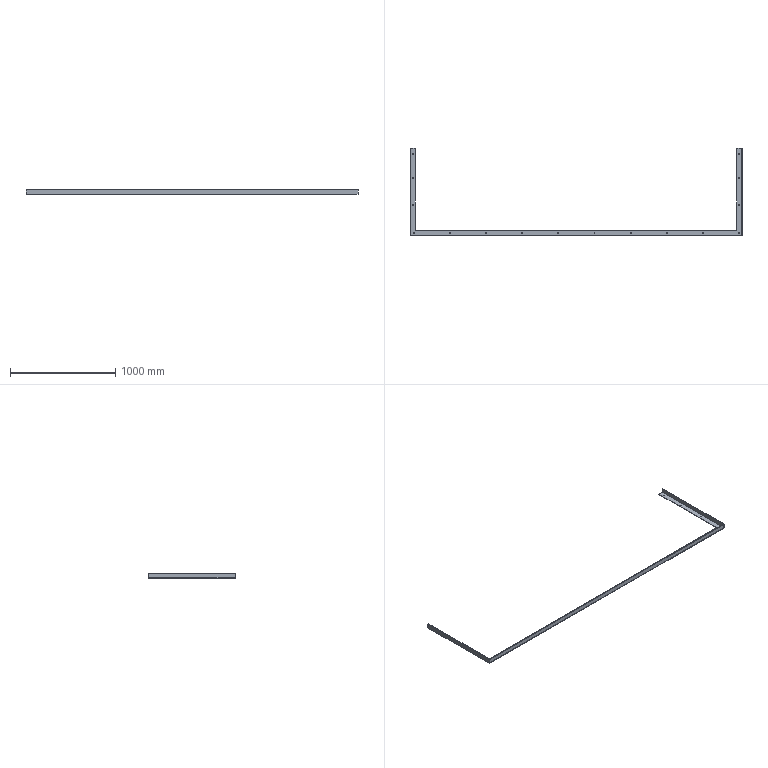Part | SolidWorks | features BaseBody 1 | 1 solid | 46 faces | box 3151 x 827 x 44 mm | volume 1704448 mm3 | cylinder 32 | plane 14 | commonest cylinder face diameters 9 x32
STEP:
#1=CARTESIAN_POINT('',(3127.5,774.,4.));
#2=VERTEX_POINT('',#1);
#3=CARTESIAN_POINT('',(3118.5,774.,4.));
#4=VERTEX_POINT('',#3);
#5=CARTESIAN_POINT('',(3123.,774.,4.));
#6=DIRECTION('',(0.,0.,-1.));
#7=DIRECTION('',(-1.,0.,0.));
#8=AXIS2_PLACEMENT_3D('',#5,#6,#7);
#9=CIRCLE('',#8,4.5);
#10=EDGE_CURVE('',#2,#4,#9,.T.);
#11=ORIENTED_EDGE('',*,*,#10,.F.);
#12=CARTESIAN_POINT('',(3127.5,774.,0.));
#13=VERTEX_POINT('',#12);
#14=CARTESIAN_POINT('',(3127.5,774.,44.));
#15=DIRECTION('',(0.,0.,-1.));
#16=VECTOR('',#15,1000.);
#17=LINE('',#14,#16);
#18=EDGE_CURVE('',#2,#13,#17,.T.);
#19=ORIENTED_EDGE('',*,*,#18,.T.);
#20=CARTESIAN_POINT('',(3118.5,774.,0.));
#21=VERTEX_POINT('',#20);
#22=CARTESIAN_POINT('',(3123.,774.,0.));
#23=DIRECTION('',(0.,0.,1.));
#24=DIRECTION('',(-1.,0.,0.));
#25=AXIS2_PLACEMENT_3D('',#22,#23,#24);
#26=CIRCLE('',#25,4.5);
#27=EDGE_CURVE('',#21,#13,#26,.T.);
#28=ORIENTED_EDGE('',*,*,#27,.F.);
#29=CARTESIAN_POINT('',(3118.5,774.,44.));
#30=DIRECTION('',(0.,0.,-1.));
#31=VECTOR('',#30,1000.);
#32=LINE('',#29,#31);
#33=EDGE_CURVE('',#4,#21,#32,.T.);
#34=ORIENTED_EDGE('',*,*,#33,.F.);
#35=EDGE_LOOP('',(#11,#19,#28,#34));
#36=FACE_OUTER_BOUND('',#35,.T.);
#37=CARTESIAN_POINT('',(3123.,774.,44.));
#38=DIRECTION('',(0.,0.,-1.));
#39=DIRECTION('',(-1.,0.,0.));
#40=AXIS2_PLACEMENT_3D('',#37,#38,#39);
#41=CYLINDRICAL_SURFACE('',#40,4.5);
#42=ADVANCED_FACE('',(#36),#41,.F.);
#43=CARTESIAN_POINT('',(32.5,774.,4.));
#44=VERTEX_POINT('',#43);
#45=CARTESIAN_POINT('',(23.5,774.,4.));
#46=VERTEX_POINT('',#45);
#47=CARTESIAN_POINT('',(28.,774.,4.));
#48=DIRECTION('',(0.,0.,-1.));
#49=DIRECTION('',(-1.,0.,0.));
#50=AXIS2_PLACEMENT_3D('',#47,#48,#49);
#51=CIRCLE('',#50,4.5);
#52=EDGE_CURVE('',#44,#46,#51,.T.);
#53=ORIENTED_EDGE('',*,*,#52,.F.);
#54=CARTESIAN_POINT('',(32.5,774.,0.));
#55=VERTEX_POINT('',#54);
#56=CARTESIAN_POINT('',(32.5,774.,44.));
#57=DIRECTION('',(0.,0.,-1.));
#58=VECTOR('',#57,1000.);
#59=LINE('',#56,#58);
#60=EDGE_CURVE('',#44,#55,#59,.T.);
#61=ORIENTED_EDGE('',*,*,#60,.T.);
#62=CARTESIAN_POINT('',(23.5,774.,0.));
#63=VERTEX_POINT('',#62);
#64=CARTESIAN_POINT('',(28.,774.,0.));
#65=DIRECTION('',(0.,0.,1.));
#66=DIRECTION('',(-1.,0.,0.));
#67=AXIS2_PLACEMENT_3D('',#64,#65,#66);
#68=CIRCLE('',#67,4.5);
#69=EDGE_CURVE('',#63,#55,#68,.T.);
#70=ORIENTED_EDGE('',*,*,#69,.F.);
#71=CARTESIAN_POINT('',(23.5,774.,44.));
#72=DIRECTION('',(0.,0.,-1.));
#73=VECTOR('',#72,1000.);
#74=LINE('',#71,#73);
#75=EDGE_CURVE('',#46,#63,#74,.T.);
#76=ORIENTED_EDGE('',*,*,#75,.F.);
#77=EDGE_LOOP('',(#53,#61,#70,#76));
#78=FACE_OUTER_BOUND('',#77,.T.);
#79=CARTESIAN_POINT('',(28.,774.,44.));
#80=DIRECTION('',(0.,0.,-1.));
#81=DIRECTION('',(-1.,0.,0.));
#82=AXIS2_PLACEMENT_3D('',#79,#80,#81);
#83=CYLINDRICAL_SURFACE('',#82,4.5);
#84=ADVANCED_FACE('',(#78),#83,.F.);
#85=CARTESIAN_POINT('',(32.5,546.,4.));
#86=VERTEX_POINT('',#85);
#87=CARTESIAN_POINT('',(23.5,546.,4.));
#88=VERTEX_POINT('',#87);
#89=CARTESIAN_POINT('',(28.,546.,4.));
#90=DIRECTION('',(0.,0.,-1.));
#91=DIRECTION('',(-1.,0.,0.));
#92=AXIS2_PLACEMENT_3D('',#89,#90,#91);
#93=CIRCLE('',#92,4.5);
#94=EDGE_CURVE('',#86,#88,#93,.T.);
#95=ORIENTED_EDGE('',*,*,#94,.F.);
#96=CARTESIAN_POINT('',(32.5,546.,0.));
#97=VERTEX_POINT('',#96);
#98=CARTESIAN_POINT('',(32.5,546.,44.));
#99=DIRECTION('',(0.,0.,-1.));
#100=VECTOR('',#99,1000.);
#101=LINE('',#98,#100);
#102=EDGE_CURVE('',#86,#97,#101,.T.);
#103=ORIENTED_EDGE('',*,*,#102,.T.);
#104=CARTESIAN_POINT('',(23.5,546.,0.));
#105=VERTEX_POINT('',#104);
#106=CARTESIAN_POINT('',(28.,546.,0.));
#107=DIRECTION('',(0.,0.,1.));
#108=DIRECTION('',(-1.,0.,0.));
#109=AXIS2_PLACEMENT_3D('',#106,#107,#108);
#110=CIRCLE('',#109,4.5);
#111=EDGE_CURVE('',#105,#97,#110,.T.);
#112=ORIENTED_EDGE('',*,*,#111,.F.);
#113=CARTESIAN_POINT('',(23.5,546.,44.));
#114=DIRECTION('',(0.,0.,-1.));
#115=VECTOR('',#114,1000.);
#116=LINE('',#113,#115);
#117=EDGE_CURVE('',#88,#105,#116,.T.);
#118=ORIENTED_EDGE('',*,*,#117,.F.);
#119=EDGE_LOOP('',(#95,#103,#112,#118));
#120=FACE_OUTER_BOUND('',#119,.T.);
#121=CARTESIAN_POINT('',(28.,546.,44.));
#122=DIRECTION('',(0.,0.,-1.));
#123=DIRECTION('',(-1.,0.,0.));
#124=AXIS2_PLACEMENT_3D('',#121,#122,#123);
#125=CYLINDRICAL_SURFACE('',#124,4.5);
#126=ADVANCED_FACE('',(#120),#125,.F.);
#127=CARTESIAN_POINT('',(32.5,286.,4.));
#128=VERTEX_POINT('',#127);
#129=CARTESIAN_POINT('',(23.5,286.,4.));
#130=VERTEX_POINT('',#129);
#131=CARTESIAN_POINT('',(28.,286.,4.));
#132=DIRECTION('',(0.,0.,-1.));
#133=DIRECTION('',(-1.,0.,0.));
#134=AXIS2_PLACEMENT_3D('',#131,#132,#133);
#135=CIRCLE('',#134,4.5);
#136=EDGE_CURVE('',#128,#130,#135,.T.);
#137=ORIENTED_EDGE('',*,*,#136,.F.);
#138=CARTESIAN_POINT('',(32.5,286.,0.));
#139=VERTEX_POINT('',#138);
#140=CARTESIAN_POINT('',(32.5,286.,44.));
#141=DIRECTION('',(0.,0.,-1.));
#142=VECTOR('',#141,1000.);
#143=LINE('',#140,#142);
#144=EDGE_CURVE('',#128,#139,#143,.T.);
#145=ORIENTED_EDGE('',*,*,#144,.T.);
#146=CARTESIAN_POINT('',(23.5,286.,0.));
#147=VERTEX_POINT('',#146);
#148=CARTESIAN_POINT('',(28.,286.,0.));
#149=DIRECTION('',(0.,0.,1.));
#150=DIRECTION('',(-1.,0.,0.));
#151=AXIS2_PLACEMENT_3D('',#148,#149,#150);
#152=CIRCLE('',#151,4.5);
#153=EDGE_CURVE('',#147,#139,#152,.T.);
#154=ORIENTED_EDGE('',*,*,#153,.F.);
#155=CARTESIAN_POINT('',(23.5,286.,44.));
#156=DIRECTION('',(0.,0.,-1.));
#157=VECTOR('',#156,1000.);
#158=LINE('',#155,#157);
#159=EDGE_CURVE('',#130,#147,#158,.T.);
#160=ORIENTED_EDGE('',*,*,#159,.F.);
#161=EDGE_LOOP('',(#137,#145,#154,#160));
#162=FACE_OUTER_BOUND('',#161,.T.);
#163=CARTESIAN_POINT('',(28.,286.,44.));
#164=DIRECTION('',(0.,0.,-1.));
#165=DIRECTION('',(-1.,0.,0.));
#166=AXIS2_PLACEMENT_3D('',#163,#164,#165);
#167=CYLINDRICAL_SURFACE('',#166,4.5);
#168=ADVANCED_FACE('',(#162),#167,.F.);
#169=CARTESIAN_POINT('',(40.5,26.,4.));
#170=VERTEX_POINT('',#169);
#171=CARTESIAN_POINT('',(31.5,26.,4.));
#172=VERTEX_POINT('',#171);
#173=CARTESIAN_POINT('',(36.,26.,4.));
#174=DIRECTION('',(0.,0.,-1.));
#175=DIRECTION('',(-1.,0.,0.));
#176=AXIS2_PLACEMENT_3D('',#173,#174,#175);
#177=CIRCLE('',#176,4.5);
#178=EDGE_CURVE('',#170,#172,#177,.T.);
#179=ORIENTED_EDGE('',*,*,#178,.F.);
#180=CARTESIAN_POINT('',(40.5,26.,0.));
#181=VERTEX_POINT('',#180);
#182=CARTESIAN_POINT('',(40.5,26.,44.));
#183=DIRECTION('',(0.,0.,-1.));
#184=VECTOR('',#183,1000.);
#185=LINE('',#182,#184);
#186=EDGE_CURVE('',#170,#181,#185,.T.);
#187=ORIENTED_EDGE('',*,*,#186,.T.);
#188=CARTESIAN_POINT('',(31.5,26.,0.));
#189=VERTEX_POINT('',#188);
#190=CARTESIAN_POINT('',(36.,26.,0.));
#191=DIRECTION('',(0.,0.,1.));
#192=DIRECTION('',(-1.,0.,0.));
#193=AXIS2_PLACEMENT_3D('',#190,#191,#192);
#194=CIRCLE('',#193,4.5);
#195=EDGE_CURVE('',#189,#181,#194,.T.);
#196=ORIENTED_EDGE('',*,*,#195,.F.);
#197=CARTESIAN_POINT('',(31.5,26.,44.));
#198=DIRECTION('',(0.,0.,-1.));
#199=VECTOR('',#198,1000.);
#200=LINE('',#197,#199);
#201=EDGE_CURVE('',#172,#189,#200,.T.);
#202=ORIENTED_EDGE('',*,*,#201,.F.);
#203=EDGE_LOOP('',(#179,#187,#196,#202));
#204=FACE_OUTER_BOUND('',#203,.T.);
#205=CARTESIAN_POINT('',(36.,26.,44.));
#206=DIRECTION('',(0.,0.,-1.));
#207=DIRECTION('',(-1.,0.,0.));
#208=AXIS2_PLACEMENT_3D('',#205,#206,#207);
#209=CYLINDRICAL_SURFACE('',#208,4.5);
#210=ADVANCED_FACE('',(#204),#209,.F.);
#211=CARTESIAN_POINT('',(3127.5,26.,4.));
#212=VERTEX_POINT('',#211);
#213=CARTESIAN_POINT('',(3118.5,26.,4.));
#214=VERTEX_POINT('',#213);
#215=CARTESIAN_POINT('',(3123.,26.,4.));
#216=DIRECTION('',(0.,0.,-1.));
#217=DIRECTION('',(-1.,0.,0.));
#218=AXIS2_PLACEMENT_3D('',#215,#216,#217);
#219=CIRCLE('',#218,4.5);
#220=EDGE_CURVE('',#212,#214,#219,.T.);
#221=ORIENTED_EDGE('',*,*,#220,.F.);
#222=CARTESIAN_POINT('',(3127.5,26.,0.));
#223=VERTEX_POINT('',#222);
#224=CARTESIAN_POINT('',(3127.5,26.,44.));
#225=DIRECTION('',(0.,0.,-1.));
#226=VECTOR('',#225,1000.);
#227=LINE('',#224,#226);
#228=EDGE_CURVE('',#212,#223,#227,.T.);
#229=ORIENTED_EDGE('',*,*,#228,.T.);
#230=CARTESIAN_POINT('',(3118.5,26.,0.));
#231=VERTEX_POINT('',#230);
#232=CARTESIAN_POINT('',(3123.,26.,0.));
#233=DIRECTION('',(0.,0.,1.));
#234=DIRECTION('',(-1.,0.,0.));
#235=AXIS2_PLACEMENT_3D('',#232,#233,#234);
#236=CIRCLE('',#235,4.5);
#237=EDGE_CURVE('',#231,#223,#236,.T.);
#238=ORIENTED_EDGE('',*,*,#237,.F.);
#239=CARTESIAN_POINT('',(3118.5,26.,44.));
#240=DIRECTION('',(0.,0.,-1.));
#241=VECTOR('',#240,1000.);
#242=LINE('',#239,#241);
#243=EDGE_CURVE('',#214,#231,#242,.T.);
#244=ORIENTED_EDGE('',*,*,#243,.F.);
#245=EDGE_LOOP('',(#221,#229,#238,#244));
#246=FACE_OUTER_BOUND('',#245,.T.);
#247=CARTESIAN_POINT('',(3123.,26.,44.));
#248=DIRECTION('',(0.,0.,-1.));
#249=DIRECTION('',(-1.,0.,0.));
#250=AXIS2_PLACEMENT_3D('',#247,#248,#249);
#251=CYLINDRICAL_SURFACE('',#250,4.5);
#252=ADVANCED_FACE('',(#246),#251,.F.);
#253=CARTESIAN_POINT('',(3127.5,286.,4.));
#254=VERTEX_POINT('',#253);
#255=CARTESIAN_POINT('',(3118.5,286.,4.));
#256=VERTEX_POINT('',#255);
#257=CARTESIAN_POINT('',(3123.,286.,4.));
#258=DIRECTION('',(0.,0.,-1.));
#259=DIRECTION('',(-1.,0.,0.));
#260=AXIS2_PLACEMENT_3D('',#257,#258,#259);
#261=CIRCLE('',#260,4.5);
#262=EDGE_CURVE('',#254,#256,#261,.T.);
#263=ORIENTED_EDGE('',*,*,#262,.F.);
#264=CARTESIAN_POINT('',(3127.5,286.,0.));
#265=VERTEX_POINT('',#264);
#266=CARTESIAN_POINT('',(3127.5,286.,44.));
#267=DIRECTION('',(0.,0.,-1.));
#268=VECTOR('',#267,1000.);
#269=LINE('',#266,#268);
#270=EDGE_CURVE('',#254,#265,#269,.T.);
#271=ORIENTED_EDGE('',*,*,#270,.T.);
#272=CARTESIAN_POINT('',(3118.5,286.,0.));
#273=VERTEX_POINT('',#272);
#274=CARTESIAN_POINT('',(3123.,286.,0.));
#275=DIRECTION('',(0.,0.,1.));
#276=DIRECTION('',(-1.,0.,0.));
#277=AXIS2_PLACEMENT_3D('',#274,#275,#276);
#278=CIRCLE('',#277,4.5);
#279=EDGE_CURVE('',#273,#265,#278,.T.);
#280=ORIENTED_EDGE('',*,*,#279,.F.);
#281=CARTESIAN_POINT('',(3118.5,286.,44.));
#282=DIRECTION('',(0.,0.,-1.));
#283=VECTOR('',#282,1000.);
#284=LINE('',#281,#283);
#285=EDGE_CURVE('',#256,#273,#284,.T.);
#286=ORIENTED_EDGE('',*,*,#285,.F.);
#287=EDGE_LOOP('',(#263,#271,#280,#286));
#288=FACE_OUTER_BOUND('',#287,.T.);
#289=CARTESIAN_POINT('',(3123.,286.,44.));
#290=DIRECTION('',(0.,0.,-1.));
#291=DIRECTION('',(-1.,0.,0.));
#292=AXIS2_PLACEMENT_3D('',#289,#290,#291);
#293=CYLINDRICAL_SURFACE('',#292,4.5);
#294=ADVANCED_FACE('',(#288),#293,.F.);
#295=CARTESIAN_POINT('',(3127.5,546.,4.));
#296=VERTEX_POINT('',#295);
#297=CARTESIAN_POINT('',(3118.5,546.,4.));
#298=VERTEX_POINT('',#297);
#299=CARTESIAN_POINT('',(3123.,546.,4.));
#300=DIRECTION('',(0.,0.,-1.));
#301=DIRECTION('',(-1.,0.,0.));
#302=AXIS2_PLACEMENT_3D('',#299,#300,#301);
#303=CIRCLE('',#302,4.5);
#304=EDGE_CURVE('',#296,#298,#303,.T.);
#305=ORIENTED_EDGE('',*,*,#304,.F.);
#306=CARTESIAN_POINT('',(3127.5,546.,0.));
#307=VERTEX_POINT('',#306);
#308=CARTESIAN_POINT('',(3127.5,546.,44.));
#309=DIRECTION('',(0.,0.,-1.));
#310=VECTOR('',#309,1000.);
#311=LINE('',#308,#310);
#312=EDGE_CURVE('',#296,#307,#311,.T.);
#313=ORIENTED_EDGE('',*,*,#312,.T.);
#314=CARTESIAN_POINT('',(3118.5,546.,0.));
#315=VERTEX_POINT('',#314);
#316=CARTESIAN_POINT('',(3123.,546.,0.));
#317=DIRECTION('',(0.,0.,1.));
#318=DIRECTION('',(-1.,0.,0.));
#319=AXIS2_PLACEMENT_3D('',#316,#317,#318);
#320=CIRCLE('',#319,4.5);
#321=EDGE_CURVE('',#315,#307,#320,.T.);
#322=ORIENTED_EDGE('',*,*,#321,.F.);
#323=CARTESIAN_POINT('',(3118.5,546.,44.));
#324=DIRECTION('',(0.,0.,-1.));
#325=VECTOR('',#324,1000.);
#326=LINE('',#323,#325);
#327=EDGE_CURVE('',#298,#315,#326,.T.);
#328=ORIENTED_EDGE('',*,*,#327,.F.);
#329=EDGE_LOOP('',(#305,#313,#322,#328));
#330=FACE_OUTER_BOUND('',#329,.T.);
#331=CARTESIAN_POINT('',(3123.,546.,44.));
#332=DIRECTION('',(0.,0.,-1.));
#333=DIRECTION('',(-1.,0.,0.));
#334=AXIS2_PLACEMENT_3D('',#331,#332,#333);
#335=CYLINDRICAL_SURFACE('',#334,4.5);
#336=ADVANCED_FACE('',(#330),#335,.F.);
#337=CARTESIAN_POINT('',(383.5,26.,4.));
#338=VERTEX_POINT('',#337);
#339=CARTESIAN_POINT('',(374.5,26.,4.));
#340=VERTEX_POINT('',#339);
#341=CARTESIAN_POINT('',(379.,26.,4.));
#342=DIRECTION('',(0.,0.,-1.));
#343=DIRECTION('',(-1.,0.,0.));
#344=AXIS2_PLACEMENT_3D('',#341,#342,#343);
#345=CIRCLE('',#344,4.5);
#346=EDGE_CURVE('',#338,#340,#345,.T.);
#347=ORIENTED_EDGE('',*,*,#346,.F.);
#348=CARTESIAN_POINT('',(383.5,26.,0.));
#349=VERTEX_POINT('',#348);
#350=CARTESIAN_POINT('',(383.5,26.,44.));
#351=DIRECTION('',(0.,0.,-1.));
#352=VECTOR('',#351,1000.);
#353=LINE('',#350,#352);
#354=EDGE_CURVE('',#338,#349,#353,.T.);
#355=ORIENTED_EDGE('',*,*,#354,.T.);
#356=CARTESIAN_POINT('',(374.5,26.,0.));
#357=VERTEX_POINT('',#356);
#358=CARTESIAN_POINT('',(379.,26.,0.));
#359=DIRECTION('',(0.,0.,1.));
#360=DIRECTION('',(-1.,0.,0.));
#361=AXIS2_PLACEMENT_3D('',#358,#359,#360);
#362=CIRCLE('',#361,4.5);
#363=EDGE_CURVE('',#357,#349,#362,.T.);
#364=ORIENTED_EDGE('',*,*,#363,.F.);
#365=CARTESIAN_POINT('',(374.5,26.,44.));
#366=DIRECTION('',(0.,0.,-1.));
#367=VECTOR('',#366,1000.);
#368=LINE('',#365,#367);
#369=EDGE_CURVE('',#340,#357,#368,.T.);
#370=ORIENTED_EDGE('',*,*,#369,.F.);
#371=EDGE_LOOP('',(#347,#355,#364,#370));
#372=FACE_OUTER_BOUND('',#371,.T.);
#373=CARTESIAN_POINT('',(379.,26.,44.));
#374=DIRECTION('',(0.,0.,-1.));
#375=DIRECTION('',(-1.,0.,0.));
#376=AXIS2_PLACEMENT_3D('',#373,#374,#375);
#377=CYLINDRICAL_SURFACE('',#376,4.5);
#378=ADVANCED_FACE('',(#372),#377,.F.);
#379=CARTESIAN_POINT('',(726.5,26.,4.));
#380=VERTEX_POINT('',#379);
#381=CARTESIAN_POINT('',(717.5,26.,4.));
#382=VERTEX_POINT('',#381);
#383=CARTESIAN_POINT('',(722.,26.,4.));
#384=DIRECTION('',(0.,0.,-1.));
#385=DIRECTION('',(-1.,0.,0.));
#386=AXIS2_PLACEMENT_3D('',#383,#384,#385);
#387=CIRCLE('',#386,4.5);
#388=EDGE_CURVE('',#380,#382,#387,.T.);
#389=ORIENTED_EDGE('',*,*,#388,.F.);
#390=CARTESIAN_POINT('',(726.5,26.,0.));
#391=VERTEX_POINT('',#390);
#392=CARTESIAN_POINT('',(726.5,26.,44.));
#393=DIRECTION('',(0.,0.,-1.));
#394=VECTOR('',#393,1000.);
#395=LINE('',#392,#394);
#396=EDGE_CURVE('',#380,#391,#395,.T.);
#397=ORIENTED_EDGE('',*,*,#396,.T.);
#398=CARTESIAN_POINT('',(717.5,26.,0.));
#399=VERTEX_POINT('',#398);
#400=CARTESIAN_POINT('',(722.,26.,0.));
#401=DIRECTION('',(0.,0.,1.));
#402=DIRECTION('',(-1.,0.,0.));
#403=AXIS2_PLACEMENT_3D('',#400,#401,#402);
#404=CIRCLE('',#403,4.5);
#405=EDGE_CURVE('',#399,#391,#404,.T.);
#406=ORIENTED_EDGE('',*,*,#405,.F.);
#407=CARTESIAN_POINT('',(717.5,26.,44.));
#408=DIRECTION('',(0.,0.,-1.));
#409=VECTOR('',#408,1000.);
#410=LINE('',#407,#409);
#411=EDGE_CURVE('',#382,#399,#410,.T.);
#412=ORIENTED_EDGE('',*,*,#411,.F.);
#413=EDGE_LOOP('',(#389,#397,#406,#412));
#414=FACE_OUTER_BOUND('',#413,.T.);
#415=CARTESIAN_POINT('',(722.,26.,44.));
#416=DIRECTION('',(0.,0.,-1.));
#417=DIRECTION('',(-1.,0.,0.));
#418=AXIS2_PLACEMENT_3D('',#415,#416,#417);
#419=CYLINDRICAL_SURFACE('',#418,4.5);
#420=ADVANCED_FACE('',(#414),#419,.F.);
#421=CARTESIAN_POINT('',(1069.5,26.,4.));
#422=VERTEX_POINT('',#421);
#423=CARTESIAN_POINT('',(1060.5,26.,4.));
#424=VERTEX_POINT('',#423);
#425=CARTESIAN_POINT('',(1065.,26.,4.));
#426=DIRECTION('',(0.,0.,-1.));
#427=DIRECTION('',(-1.,0.,0.));
#428=AXIS2_PLACEMENT_3D('',#425,#426,#427);
#429=CIRCLE('',#428,4.5);
#430=EDGE_CURVE('',#422,#424,#429,.T.);
#431=ORIENTED_EDGE('',*,*,#430,.F.);
#432=CARTESIAN_POINT('',(1069.5,26.,0.));
#433=VERTEX_POINT('',#432);
#434=CARTESIAN_POINT('',(1069.5,26.,44.));
#435=DIRECTION('',(0.,0.,-1.));
#436=VECTOR('',#435,1000.);
#437=LINE('',#434,#436);
#438=EDGE_CURVE('',#422,#433,#437,.T.);
#439=ORIENTED_EDGE('',*,*,#438,.T.);
#440=CARTESIAN_POINT('',(1060.5,26.,0.));
#441=VERTEX_POINT('',#440);
#442=CARTESIAN_POINT('',(1065.,26.,0.));
#443=DIRECTION('',(0.,0.,1.));
#444=DIRECTION('',(-1.,0.,0.));
#445=AXIS2_PLACEMENT_3D('',#442,#443,#444);
#446=CIRCLE('',#445,4.5);
#447=EDGE_CURVE('',#441,#433,#446,.T.);
#448=ORIENTED_EDGE('',*,*,#447,.F.);
#449=CARTESIAN_POINT('',(1060.5,26.,44.));
#450=DIRECTION('',(0.,0.,-1.));
#451=VECTOR('',#450,1000.);
#452=LINE('',#449,#451);
#453=EDGE_CURVE('',#424,#441,#452,.T.);
#454=ORIENTED_EDGE('',*,*,#453,.F.);
#455=EDGE_LOOP('',(#431,#439,#448,#454));
#456=FACE_OUTER_BOUND('',#455,.T.);
#457=CARTESIAN_POINT('',(1065.,26.,44.));
#458=DIRECTION('',(0.,0.,-1.));
#459=DIRECTION('',(-1.,0.,0.));
#460=AXIS2_PLACEMENT_3D('',#457,#458,#459);
#461=CYLINDRICAL_SURFACE('',#460,4.5);
#462=ADVANCED_FACE('',(#456),#461,.F.);
#463=CARTESIAN_POINT('',(1412.5,26.,4.));
#464=VERTEX_POINT('',#463);
#465=CARTESIAN_POINT('',(1403.5,26.,4.));
#466=VERTEX_POINT('',#465);
#467=CARTESIAN_POINT('',(1408.,26.,4.));
#468=DIRECTION('',(0.,0.,-1.));
#469=DIRECTION('',(-1.,0.,0.));
#470=AXIS2_PLACEMENT_3D('',#467,#468,#469);
#471=CIRCLE('',#470,4.5);
#472=EDGE_CURVE('',#464,#466,#471,.T.);
#473=ORIENTED_EDGE('',*,*,#472,.F.);
#474=CARTESIAN_POINT('',(1412.5,26.,0.));
#475=VERTEX_POINT('',#474);
#476=CARTESIAN_POINT('',(1412.5,26.,44.));
#477=DIRECTION('',(0.,0.,-1.));
#478=VECTOR('',#477,1000.);
#479=LINE('',#476,#478);
#480=EDGE_CURVE('',#464,#475,#479,.T.);
#481=ORIENTED_EDGE('',*,*,#480,.T.);
#482=CARTESIAN_POINT('',(1403.5,26.,0.));
#483=VERTEX_POINT('',#482);
#484=CARTESIAN_POINT('',(1408.,26.,0.));
#485=DIRECTION('',(0.,0.,1.));
#486=DIRECTION('',(-1.,0.,0.));
#487=AXIS2_PLACEMENT_3D('',#484,#485,#486);
#488=CIRCLE('',#487,4.5);
#489=EDGE_CURVE('',#483,#475,#488,.T.);
#490=ORIENTED_EDGE('',*,*,#489,.F.);
#491=CARTESIAN_POINT('',(1403.5,26.,44.));
#492=DIRECTION('',(0.,0.,-1.));
#493=VECTOR('',#492,1000.);
#494=LINE('',#491,#493);
#495=EDGE_CURVE('',#466,#483,#494,.T.);
#496=ORIENTED_EDGE('',*,*,#495,.F.);
#497=EDGE_LOOP('',(#473,#481,#490,#496));
#498=FACE_OUTER_BOUND('',#497,.T.);
#499=CARTESIAN_POINT('',(1408.,26.,44.));
#500=DIRECTION('',(0.,0.,-1.));
#501=DIRECTION('',(-1.,0.,0.));
#502=AXIS2_PLACEMENT_3D('',#499,#500,#501);
#503=CYLINDRICAL_SURFACE('',#502,4.5);
#504=ADVANCED_FACE('',(#498),#503,.F.);
#505=CARTESIAN_POINT('',(1755.5,26.,4.));
#506=VERTEX_POINT('',#505);
#507=CARTESIAN_POINT('',(1746.5,26.,4.));
#508=VERTEX_POINT('',#507);
#509=CARTESIAN_POINT('',(1751.,26.,4.));
#510=DIRECTION('',(0.,0.,-1.));
#511=DIRECTION('',(-1.,0.,0.));
#512=AXIS2_PLACEMENT_3D('',#509,#510,#511);
#513=CIRCLE('',#512,4.5);
#514=EDGE_CURVE('',#506,#508,#513,.T.);
#515=ORIENTED_EDGE('',*,*,#514,.F.);
#516=CARTESIAN_POINT('',(1755.5,26.,0.));
#517=VERTEX_POINT('',#516);
#518=CARTESIAN_POINT('',(1755.5,26.,44.));
#519=DIRECTION('',(0.,0.,-1.));
#520=VECTOR('',#519,1000.);
#521=LINE('',#518,#520);
#522=EDGE_CURVE('',#506,#517,#521,.T.);
#523=ORIENTED_EDGE('',*,*,#522,.T.);
#524=CARTESIAN_POINT('',(1746.5,26.,0.));
#525=VERTEX_POINT('',#524);
#526=CARTESIAN_POINT('',(1751.,26.,0.));
#527=DIRECTION('',(0.,0.,1.));
#528=DIRECTION('',(-1.,0.,0.));
#529=AXIS2_PLACEMENT_3D('',#526,#527,#528);
#530=CIRCLE('',#529,4.5);
#531=EDGE_CURVE('',#525,#517,#530,.T.);
#532=ORIENTED_EDGE('',*,*,#531,.F.);
#533=CARTESIAN_POINT('',(1746.5,26.,44.));
#534=DIRECTION('',(0.,0.,-1.));
#535=VECTOR('',#534,1000.);
#536=LINE('',#533,#535);
#537=EDGE_CURVE('',#508,#525,#536,.T.);
#538=ORIENTED_EDGE('',*,*,#537,.F.);
#539=EDGE_LOOP('',(#515,#523,#532,#538));
#540=FACE_OUTER_BOUND('',#539,.T.);
#541=CARTESIAN_POINT('',(1751.,26.,44.));
#542=DIRECTION('',(0.,0.,-1.));
#543=DIRECTION('',(-1.,0.,0.));
#544=AXIS2_PLACEMENT_3D('',#541,#542,#543);
#545=CYLINDRICAL_SURFACE('',#544,4.5);
#546=ADVANCED_FACE('',(#540),#545,.F.);
#547=CARTESIAN_POINT('',(2098.5,26.,4.));
#548=VERTEX_POINT('',#547);
#549=CARTESIAN_POINT('',(2089.5,26.,4.));
#550=VERTEX_POINT('',#549);
#551=CARTESIAN_POINT('',(2094.,26.,4.));
#552=DIRECTION('',(0.,0.,-1.));
#553=DIRECTION('',(-1.,0.,0.));
#554=AXIS2_PLACEMENT_3D('',#551,#552,#553);
#555=CIRCLE('',#554,4.5);
#556=EDGE_CURVE('',#548,#550,#555,.T.);
#557=ORIENTED_EDGE('',*,*,#556,.F.);
#558=CARTESIAN_POINT('',(2098.5,26.,0.));
#559=VERTEX_POINT('',#558);
#560=CARTESIAN_POINT('',(2098.5,26.,44.));
#561=DIRECTION('',(0.,0.,-1.));
#562=VECTOR('',#561,1000.);
#563=LINE('',#560,#562);
#564=EDGE_CURVE('',#548,#559,#563,.T.);
#565=ORIENTED_EDGE('',*,*,#564,.T.);
#566=CARTESIAN_POINT('',(2089.5,26.,0.));
#567=VERTEX_POINT('',#566);
#568=CARTESIAN_POINT('',(2094.,26.,0.));
#569=DIRECTION('',(0.,0.,1.));
#570=DIRECTION('',(-1.,0.,0.));
#571=AXIS2_PLACEMENT_3D('',#568,#569,#570);
#572=CIRCLE('',#571,4.5);
#573=EDGE_CURVE('',#567,#559,#572,.T.);
#574=ORIENTED_EDGE('',*,*,#573,.F.);
#575=CARTESIAN_POINT('',(2089.5,26.,44.));
#576=DIRECTION('',(0.,0.,-1.));
#577=VECTOR('',#576,1000.);
#578=LINE('',#575,#577);
#579=EDGE_CURVE('',#550,#567,#578,.T.);
#580=ORIENTED_EDGE('',*,*,#579,.F.);
#581=EDGE_LOOP('',(#557,#565,#574,#580));
#582=FACE_OUTER_BOUND('',#581,.T.);
#583=CARTESIAN_POINT('',(2094.,26.,44.));
#584=DIRECTION('',(0.,0.,-1.));
#585=DIRECTION('',(-1.,0.,0.));
#586=AXIS2_PLACEMENT_3D('',#583,#584,#585);
#587=CYLINDRICAL_SURFACE('',#586,4.5);
#588=ADVANCED_FACE('',(#582),#587,.F.);
#589=CARTESIAN_POINT('',(2441.5,26.,4.));
#590=VERTEX_POINT('',#589);
#591=CARTESIAN_POINT('',(2432.5,26.,4.));
#592=VERTEX_POINT('',#591);
#593=CARTESIAN_POINT('',(2437.,26.,4.));
#594=DIRECTION('',(0.,0.,-1.));
#595=DIRECTION('',(-1.,0.,0.));
#596=AXIS2_PLACEMENT_3D('',#593,#594,#595);
#597=CIRCLE('',#596,4.5);
#598=EDGE_CURVE('',#590,#592,#597,.T.);
#599=ORIENTED_EDGE('',*,*,#598,.F.);
#600=CARTESIAN_POINT('',(2441.5,26.,0.));
#601=VERTEX_POINT('',#600);
#602=CARTESIAN_POINT('',(2441.5,26.,44.));
#603=DIRECTION('',(0.,0.,-1.));
#604=VECTOR('',#603,1000.);
#605=LINE('',#602,#604);
#606=EDGE_CURVE('',#590,#601,#605,.T.);
#607=ORIENTED_EDGE('',*,*,#606,.T.);
#608=CARTESIAN_POINT('',(2432.5,26.,0.));
#609=VERTEX_POINT('',#608);
#610=CARTESIAN_POINT('',(2437.,26.,0.));
#611=DIRECTION('',(0.,0.,1.));
#612=DIRECTION('',(-1.,0.,0.));
#613=AXIS2_PLACEMENT_3D('',#610,#611,#612);
#614=CIRCLE('',#613,4.5);
#615=EDGE_CURVE('',#609,#601,#614,.T.);
#616=ORIENTED_EDGE('',*,*,#615,.F.);
#617=CARTESIAN_POINT('',(2432.5,26.,44.));
#618=DIRECTION('',(0.,0.,-1.));
#619=VECTOR('',#618,1000.);
#620=LINE('',#617,#619);
#621=EDGE_CURVE('',#592,#609,#620,.T.);
#622=ORIENTED_EDGE('',*,*,#621,.F.);
#623=EDGE_LOOP('',(#599,#607,#616,#622));
#624=FACE_OUTER_BOUND('',#623,.T.);
#625=CARTESIAN_POINT('',(2437.,26.,44.));
#626=DIRECTION('',(0.,0.,-1.));
#627=DIRECTION('',(-1.,0.,0.));
#628=AXIS2_PLACEMENT_3D('',#625,#626,#627);
#629=CYLINDRICAL_SURFACE('',#628,4.5);
#630=ADVANCED_FACE('',(#624),#629,.F.);
#631=CARTESIAN_POINT('',(2784.5,26.,4.));
#632=VERTEX_POINT('',#631);
#633=CARTESIAN_POINT('',(2775.5,26.,4.));
#634=VERTEX_POINT('',#633);
#635=CARTESIAN_POINT('',(2780.,26.,4.));
#636=DIRECTION('',(0.,0.,-1.));
#637=DIRECTION('',(-1.,0.,0.));
#638=AXIS2_PLACEMENT_3D('',#635,#636,#637);
#639=CIRCLE('',#638,4.5);
#640=EDGE_CURVE('',#632,#634,#639,.T.);
#641=ORIENTED_EDGE('',*,*,#640,.F.);
#642=CARTESIAN_POINT('',(2784.5,26.,0.));
#643=VERTEX_POINT('',#642);
#644=CARTESIAN_POINT('',(2784.5,26.,44.));
#645=DIRECTION('',(0.,0.,-1.));
#646=VECTOR('',#645,1000.);
#647=LINE('',#644,#646);
#648=EDGE_CURVE('',#632,#643,#647,.T.);
#649=ORIENTED_EDGE('',*,*,#648,.T.);
#650=CARTESIAN_POINT('',(2775.5,26.,0.));
#651=VERTEX_POINT('',#650);
#652=CARTESIAN_POINT('',(2780.,26.,0.));
#653=DIRECTION('',(0.,0.,1.));
#654=DIRECTION('',(-1.,0.,0.));
#655=AXIS2_PLACEMENT_3D('',#652,#653,#654);
#656=CIRCLE('',#655,4.5);
#657=EDGE_CURVE('',#651,#643,#656,.T.);
#658=ORIENTED_EDGE('',*,*,#657,.F.);
#659=CARTESIAN_POINT('',(2775.5,26.,44.));
#660=DIRECTION('',(0.,0.,-1.));
#661=VECTOR('',#660,1000.);
#662=LINE('',#659,#661);
#663=EDGE_CURVE('',#634,#651,#662,.T.);
#664=ORIENTED_EDGE('',*,*,#663,.F.);
#665=EDGE_LOOP('',(#641,#649,#658,#664));
#666=FACE_OUTER_BOUND('',#665,.T.);
#667=CARTESIAN_POINT('',(2780.,26.,44.));
#668=DIRECTION('',(0.,0.,-1.));
#669=DIRECTION('',(-1.,0.,0.));
#670=AXIS2_PLACEMENT_3D('',#667,#668,#669);
#671=CYLINDRICAL_SURFACE('',#670,4.5);
#672=ADVANCED_FACE('',(#666),#671,.F.);
#673=CARTESIAN_POINT('',(3101.,827.,0.));
#674=VERTEX_POINT('',#673);
#675=CARTESIAN_POINT('',(3151.,827.,0.));
#676=VERTEX_POINT('',#675);
#677=CARTESIAN_POINT('',(0.,827.,0.));
#678=DIRECTION('',(1.,0.,0.));
#679=VECTOR('',#678,1000.);
#680=LINE('',#677,#679);
#681=EDGE_CURVE('',#674,#676,#680,.T.);
#682=ORIENTED_EDGE('',*,*,#681,.T.);
#683=CARTESIAN_POINT('',(3151.,0.,0.));
#684=VERTEX_POINT('',#683);
#685=CARTESIAN_POINT('',(3151.,0.,0.));
#686=DIRECTION('',(0.,-1.,0.));
#687=VECTOR('',#686,1000.);
#688=LINE('',#685,#687);
#689=EDGE_CURVE('',#676,#684,#688,.T.);
#690=ORIENTED_EDGE('',*,*,#689,.T.);
#691=CARTESIAN_POINT('',(0.,0.,0.));
#692=VERTEX_POINT('',#691);
#693=CARTESIAN_POINT('',(0.,0.,0.));
#694=DIRECTION('',(-1.,0.,0.));
#695=VECTOR('',#694,1000.);
#696=LINE('',#693,#695);
#697=EDGE_CURVE('',#684,#692,#696,.T.);
#698=ORIENTED_EDGE('',*,*,#697,.T.);
#699=CARTESIAN_POINT('',(0.,827.,0.));
#700=VERTEX_POINT('',#699);
#701=CARTESIAN_POINT('',(0.,0.,0.));
#702=DIRECTION('',(0.,1.,0.));
#703=VECTOR('',#702,1000.);
#704=LINE('',#701,#703);
#705=EDGE_CURVE('',#692,#700,#704,.T.);
#706=ORIENTED_EDGE('',*,*,#705,.T.);
#707=CARTESIAN_POINT('',(50.,827.,0.));
#708=VERTEX_POINT('',#707);
#709=CARTESIAN_POINT('',(0.,827.,0.));
#710=DIRECTION('',(1.,0.,0.));
#711=VECTOR('',#710,1000.);
#712=LINE('',#709,#711);
#713=EDGE_CURVE('',#700,#708,#712,.T.);
#714=ORIENTED_EDGE('',*,*,#713,.T.);
#715=CARTESIAN_POINT('',(50.,50.,0.));
#716=VERTEX_POINT('',#715);
#717=CARTESIAN_POINT('',(50.,0.,0.));
#718=DIRECTION('',(0.,-1.,0.));
#719=VECTOR('',#718,1000.);
#720=LINE('',#717,#719);
#721=EDGE_CURVE('',#708,#716,#720,.T.);
#722=ORIENTED_EDGE('',*,*,#721,.T.);
#723=CARTESIAN_POINT('',(3101.,50.,0.));
#724=VERTEX_POINT('',#723);
#725=CARTESIAN_POINT('',(0.,50.,0.));
#726=DIRECTION('',(1.,0.,0.));
#727=VECTOR('',#726,1000.);
#728=LINE('',#725,#727);
#729=EDGE_CURVE('',#716,#724,#728,.T.);
#730=ORIENTED_EDGE('',*,*,#729,.T.);
#731=CARTESIAN_POINT('',(3101.,0.,0.));
#732=DIRECTION('',(0.,1.,0.));
#733=VECTOR('',#732,1000.);
#734=LINE('',#731,#733);
#735=EDGE_CURVE('',#724,#674,#734,.T.);
#736=ORIENTED_EDGE('',*,*,#735,.T.);
#737=EDGE_LOOP('',(#682,#690,#698,#706,#714,#722,#730,#736));
#738=FACE_OUTER_BOUND('',#737,.T.);
#739=ORIENTED_EDGE('',*,*,#27,.T.);
#740=CARTESIAN_POINT('',(3123.,774.,0.));
#741=DIRECTION('',(0.,0.,1.));
#742=DIRECTION('',(-1.,0.,0.));
#743=AXIS2_PLACEMENT_3D('',#740,#741,#742);
#744=CIRCLE('',#743,4.5);
#745=EDGE_CURVE('',#13,#21,#744,.T.);
#746=ORIENTED_EDGE('',*,*,#745,.T.);
#747=EDGE_LOOP('',(#739,#746));
#748=FACE_BOUND('',#747,.T.);
#749=ORIENTED_EDGE('',*,*,#69,.T.);
#750=CARTESIAN_POINT('',(28.,774.,0.));
#751=DIRECTION('',(0.,0.,1.));
#752=DIRECTION('',(-1.,0.,0.));
#753=AXIS2_PLACEMENT_3D('',#750,#751,#752);
#754=CIRCLE('',#753,4.5);
#755=EDGE_CURVE('',#55,#63,#754,.T.);
#756=ORIENTED_EDGE('',*,*,#755,.T.);
#757=EDGE_LOOP('',(#749,#756));
#758=FACE_BOUND('',#757,.T.);
#759=ORIENTED_EDGE('',*,*,#111,.T.);
#760=CARTESIAN_POINT('',(28.,546.,0.));
#761=DIRECTION('',(0.,0.,1.));
#762=DIRECTION('',(-1.,0.,0.));
#763=AXIS2_PLACEMENT_3D('',#760,#761,#762);
#764=CIRCLE('',#763,4.5);
#765=EDGE_CURVE('',#97,#105,#764,.T.);
#766=ORIENTED_EDGE('',*,*,#765,.T.);
#767=EDGE_LOOP('',(#759,#766));
#768=FACE_BOUND('',#767,.T.);
#769=ORIENTED_EDGE('',*,*,#153,.T.);
#770=CARTESIAN_POINT('',(28.,286.,0.));
#771=DIRECTION('',(0.,0.,1.));
#772=DIRECTION('',(-1.,0.,0.));
#773=AXIS2_PLACEMENT_3D('',#770,#771,#772);
#774=CIRCLE('',#773,4.5);
#775=EDGE_CURVE('',#139,#147,#774,.T.);
#776=ORIENTED_EDGE('',*,*,#775,.T.);
#777=EDGE_LOOP('',(#769,#776));
#778=FACE_BOUND('',#777,.T.);
#779=ORIENTED_EDGE('',*,*,#195,.T.);
#780=CARTESIAN_POINT('',(36.,26.,0.));
#781=DIRECTION('',(0.,0.,1.));
#782=DIRECTION('',(-1.,0.,0.));
#783=AXIS2_PLACEMENT_3D('',#780,#781,#782);
#784=CIRCLE('',#783,4.5);
#785=EDGE_CURVE('',#181,#189,#784,.T.);
#786=ORIENTED_EDGE('',*,*,#785,.T.);
#787=EDGE_LOOP('',(#779,#786));
#788=FACE_BOUND('',#787,.T.);
#789=ORIENTED_EDGE('',*,*,#237,.T.);
#790=CARTESIAN_POINT('',(3123.,26.,0.));
#791=DIRECTION('',(0.,0.,1.));
#792=DIRECTION('',(-1.,0.,0.));
#793=AXIS2_PLACEMENT_3D('',#790,#791,#792);
#794=CIRCLE('',#793,4.5);
#795=EDGE_CURVE('',#223,#231,#794,.T.);
#796=ORIENTED_EDGE('',*,*,#795,.T.);
#797=EDGE_LOOP('',(#789,#796));
#798=FACE_BOUND('',#797,.T.);
#799=ORIENTED_EDGE('',*,*,#279,.T.);
#800=CARTESIAN_POINT('',(3123.,286.,0.));
#801=DIRECTION('',(0.,0.,1.));
#802=DIRECTION('',(-1.,0.,0.));
#803=AXIS2_PLACEMENT_3D('',#800,#801,#802);
#804=CIRCLE('',#803,4.5);
#805=EDGE_CURVE('',#265,#273,#804,.T.);
#806=ORIENTED_EDGE('',*,*,#805,.T.);
#807=EDGE_LOOP('',(#799,#806));
#808=FACE_BOUND('',#807,.T.);
#809=ORIENTED_EDGE('',*,*,#321,.T.);
#810=CARTESIAN_POINT('',(3123.,546.,0.));
#811=DIRECTION('',(0.,0.,1.));
#812=DIRECTION('',(-1.,0.,0.));
#813=AXIS2_PLACEMENT_3D('',#810,#811,#812);
#814=CIRCLE('',#813,4.5);
#815=EDGE_CURVE('',#307,#315,#814,.T.);
#816=ORIENTED_EDGE('',*,*,#815,.T.);
#817=EDGE_LOOP('',(#809,#816));
#818=FACE_BOUND('',#817,.T.);
#819=ORIENTED_EDGE('',*,*,#363,.T.);
#820=CARTESIAN_POINT('',(379.,26.,0.));
#821=DIRECTION('',(0.,0.,1.));
#822=DIRECTION('',(-1.,0.,0.));
#823=AXIS2_PLACEMENT_3D('',#820,#821,#822);
#824=CIRCLE('',#823,4.5);
#825=EDGE_CURVE('',#349,#357,#824,.T.);
#826=ORIENTED_EDGE('',*,*,#825,.T.);
#827=EDGE_LOOP('',(#819,#826));
#828=FACE_BOUND('',#827,.T.);
#829=ORIENTED_EDGE('',*,*,#405,.T.);
#830=CARTESIAN_POINT('',(722.,26.,0.));
#831=DIRECTION('',(0.,0.,1.));
#832=DIRECTION('',(-1.,0.,0.));
#833=AXIS2_PLACEMENT_3D('',#830,#831,#832);
#834=CIRCLE('',#833,4.5);
#835=EDGE_CURVE('',#391,#399,#834,.T.);
#836=ORIENTED_EDGE('',*,*,#835,.T.);
#837=EDGE_LOOP('',(#829,#836));
#838=FACE_BOUND('',#837,.T.);
#839=ORIENTED_EDGE('',*,*,#447,.T.);
#840=CARTESIAN_POINT('',(1065.,26.,0.));
#841=DIRECTION('',(0.,0.,1.));
#842=DIRECTION('',(-1.,0.,0.));
#843=AXIS2_PLACEMENT_3D('',#840,#841,#842);
#844=CIRCLE('',#843,4.5);
#845=EDGE_CURVE('',#433,#441,#844,.T.);
#846=ORIENTED_EDGE('',*,*,#845,.T.);
#847=EDGE_LOOP('',(#839,#846));
#848=FACE_BOUND('',#847,.T.);
#849=ORIENTED_EDGE('',*,*,#489,.T.);
#850=CARTESIAN_POINT('',(1408.,26.,0.));
#851=DIRECTION('',(0.,0.,1.));
#852=DIRECTION('',(-1.,0.,0.));
#853=AXIS2_PLACEMENT_3D('',#850,#851,#852);
#854=CIRCLE('',#853,4.5);
#855=EDGE_CURVE('',#475,#483,#854,.T.);
#856=ORIENTED_EDGE('',*,*,#855,.T.);
#857=EDGE_LOOP('',(#849,#856));
#858=FACE_BOUND('',#857,.T.);
#859=ORIENTED_EDGE('',*,*,#531,.T.);
#860=CARTESIAN_POINT('',(1751.,26.,0.));
#861=DIRECTION('',(0.,0.,1.));
#862=DIRECTION('',(-1.,0.,0.));
#863=AXIS2_PLACEMENT_3D('',#860,#861,#862);
#864=CIRCLE('',#863,4.5);
#865=EDGE_CURVE('',#517,#525,#864,.T.);
#866=ORIENTED_EDGE('',*,*,#865,.T.);
#867=EDGE_LOOP('',(#859,#866));
#868=FACE_BOUND('',#867,.T.);
#869=ORIENTED_EDGE('',*,*,#573,.T.);
#870=CARTESIAN_POINT('',(2094.,26.,0.));
#871=DIRECTION('',(0.,0.,1.));
#872=DIRECTION('',(-1.,0.,0.));
#873=AXIS2_PLACEMENT_3D('',#870,#871,#872);
#874=CIRCLE('',#873,4.5);
#875=EDGE_CURVE('',#559,#567,#874,.T.);
#876=ORIENTED_EDGE('',*,*,#875,.T.);
#877=EDGE_LOOP('',(#869,#876));
#878=FACE_BOUND('',#877,.T.);
#879=ORIENTED_EDGE('',*,*,#615,.T.);
#880=CARTESIAN_POINT('',(2437.,26.,0.));
#881=DIRECTION('',(0.,0.,1.));
#882=DIRECTION('',(-1.,0.,0.));
#883=AXIS2_PLACEMENT_3D('',#880,#881,#882);
#884=CIRCLE('',#883,4.5);
#885=EDGE_CURVE('',#601,#609,#884,.T.);
#886=ORIENTED_EDGE('',*,*,#885,.T.);
#887=EDGE_LOOP('',(#879,#886));
#888=FACE_BOUND('',#887,.T.);
#889=ORIENTED_EDGE('',*,*,#657,.T.);
#890=CARTESIAN_POINT('',(2780.,26.,0.));
#891=DIRECTION('',(0.,0.,1.));
#892=DIRECTION('',(-1.,0.,0.));
#893=AXIS2_PLACEMENT_3D('',#890,#891,#892);
#894=CIRCLE('',#893,4.5);
#895=EDGE_CURVE('',#643,#651,#894,.T.);
#896=ORIENTED_EDGE('',*,*,#895,.T.);
#897=EDGE_LOOP('',(#889,#896));
#898=FACE_BOUND('',#897,.T.);
#899=CARTESIAN_POINT('',(0.,0.,0.));
#900=DIRECTION('',(0.,0.,-1.));
#901=DIRECTION('',(-1.,0.,0.));
#902=AXIS2_PLACEMENT_3D('',#899,#900,#901);
#903=PLANE('',#902);
#904=ADVANCED_FACE('',(#738,#748,#758,#768,#778,#788,#798,#808,#818,#828,#838,#848,#858,#868,#878,#888,#898),#903,.T.);
#905=CARTESIAN_POINT('',(3151.,827.,44.));
#906=VERTEX_POINT('',#905);
#907=CARTESIAN_POINT('',(3151.,827.,4.));
#908=DIRECTION('',(0.,0.,-1.));
#909=VECTOR('',#908,1000.);
#910=LINE('',#907,#909);
#911=EDGE_CURVE('',#906,#676,#910,.T.);
#912=ORIENTED_EDGE('',*,*,#911,.F.);
#913=CARTESIAN_POINT('',(3151.,0.,44.));
#914=VERTEX_POINT('',#913);
#915=CARTESIAN_POINT('',(3151.,827.,44.));
#916=DIRECTION('',(0.,1.,0.));
#917=VECTOR('',#916,1000.);
#918=LINE('',#915,#917);
#919=EDGE_CURVE('',#914,#906,#918,.T.);
#920=ORIENTED_EDGE('',*,*,#919,.F.);
#921=CARTESIAN_POINT('',(3151.,0.,4.));
#922=DIRECTION('',(0.,0.,1.));
#923=VECTOR('',#922,1000.);
#924=LINE('',#921,#923);
#925=EDGE_CURVE('',#684,#914,#924,.T.);
#926=ORIENTED_EDGE('',*,*,#925,.F.);
#927=ORIENTED_EDGE('',*,*,#689,.F.);
#928=EDGE_LOOP('',(#912,#920,#926,#927));
#929=FACE_OUTER_BOUND('',#928,.T.);
#930=CARTESIAN_POINT('',(3151.,827.,4.));
#931=DIRECTION('',(-1.,0.,0.));
#932=DIRECTION('',(0.,0.,1.));
#933=AXIS2_PLACEMENT_3D('',#930,#931,#932);
#934=PLANE('',#933);
#935=ADVANCED_FACE('',(#929),#934,.F.);
#936=CARTESIAN_POINT('',(3101.,827.,4.));
#937=VERTEX_POINT('',#936);
#938=CARTESIAN_POINT('',(3101.,827.,4.));
#939=DIRECTION('',(0.,0.,-1.));
#940=VECTOR('',#939,1000.);
#941=LINE('',#938,#940);
#942=EDGE_CURVE('',#937,#674,#941,.T.);
#943=ORIENTED_EDGE('',*,*,#942,.F.);
#944=CARTESIAN_POINT('',(3147.,827.,4.));
#945=VERTEX_POINT('',#944);
#946=CARTESIAN_POINT('',(3101.,827.,4.));
#947=DIRECTION('',(-1.,0.,0.));
#948=VECTOR('',#947,1000.);
#949=LINE('',#946,#948);
#950=EDGE_CURVE('',#945,#937,#949,.T.);
#951=ORIENTED_EDGE('',*,*,#950,.F.);
#952=CARTESIAN_POINT('',(3147.,827.,44.));
#953=VERTEX_POINT('',#952);
#954=CARTESIAN_POINT('',(3147.,827.,4.));
#955=DIRECTION('',(0.,0.,-1.));
#956=VECTOR('',#955,1000.);
#957=LINE('',#954,#956);
#958=EDGE_CURVE('',#953,#945,#957,.T.);
#959=ORIENTED_EDGE('',*,*,#958,.F.);
#960=CARTESIAN_POINT('',(3101.,827.,44.));
#961=DIRECTION('',(-1.,0.,0.));
#962=VECTOR('',#961,1000.);
#963=LINE('',#960,#962);
#964=EDGE_CURVE('',#906,#953,#963,.T.);
#965=ORIENTED_EDGE('',*,*,#964,.F.);
#966=ORIENTED_EDGE('',*,*,#911,.T.);
#967=ORIENTED_EDGE('',*,*,#681,.F.);
#968=EDGE_LOOP('',(#943,#951,#959,#965,#966,#967));
#969=FACE_OUTER_BOUND('',#968,.T.);
#970=CARTESIAN_POINT('',(3101.,827.,4.));
#971=DIRECTION('',(0.,-1.,0.));
#972=DIRECTION('',(0.,0.,-1.));
#973=AXIS2_PLACEMENT_3D('',#970,#971,#972);
#974=PLANE('',#973);
#975=ADVANCED_FACE('',(#969),#974,.F.);
#976=CARTESIAN_POINT('',(3101.,50.,4.));
#977=VERTEX_POINT('',#976);
#978=CARTESIAN_POINT('',(3101.,50.,4.));
#979=DIRECTION('',(0.,0.,-1.));
#980=VECTOR('',#979,1000.);
#981=LINE('',#978,#980);
#982=EDGE_CURVE('',#977,#724,#981,.T.);
#983=ORIENTED_EDGE('',*,*,#982,.F.);
#984=CARTESIAN_POINT('',(3101.,50.,4.));
#985=DIRECTION('',(0.,-1.,0.));
#986=VECTOR('',#985,1000.);
#987=LINE('',#984,#986);
#988=EDGE_CURVE('',#937,#977,#987,.T.);
#989=ORIENTED_EDGE('',*,*,#988,.F.);
#990=ORIENTED_EDGE('',*,*,#942,.T.);
#991=ORIENTED_EDGE('',*,*,#735,.F.);
#992=EDGE_LOOP('',(#983,#989,#990,#991));
#993=FACE_OUTER_BOUND('',#992,.T.);
#994=CARTESIAN_POINT('',(3101.,50.,4.));
#995=DIRECTION('',(1.,0.,0.));
#996=DIRECTION('',(0.,0.,-1.));
#997=AXIS2_PLACEMENT_3D('',#994,#995,#996);
#998=PLANE('',#997);
#999=ADVANCED_FACE('',(#993),#998,.F.);
#1000=CARTESIAN_POINT('',(50.,50.,4.));
#1001=VERTEX_POINT('',#1000);
#1002=CARTESIAN_POINT('',(50.,50.,4.));
#1003=DIRECTION('',(0.,0.,-1.));
#1004=VECTOR('',#1003,1000.);
#1005=LINE('',#1002,#1004);
#1006=EDGE_CURVE('',#1001,#716,#1005,.T.);
#1007=ORIENTED_EDGE('',*,*,#1006,.F.);
#1008=CARTESIAN_POINT('',(50.,50.,4.));
#1009=DIRECTION('',(-1.,0.,0.));
#1010=VECTOR('',#1009,1000.);
#1011=LINE('',#1008,#1010);
#1012=EDGE_CURVE('',#977,#1001,#1011,.T.);
#1013=ORIENTED_EDGE('',*,*,#1012,.F.);
#1014=ORIENTED_EDGE('',*,*,#982,.T.);
#1015=ORIENTED_EDGE('',*,*,#729,.F.);
#1016=EDGE_LOOP('',(#1007,#1013,#1014,#1015));
#1017=FACE_OUTER_BOUND('',#1016,.T.);
#1018=CARTESIAN_POINT('',(50.,50.,4.));
#1019=DIRECTION('',(0.,-1.,0.));
#1020=DIRECTION('',(1.,0.,0.));
#1021=AXIS2_PLACEMENT_3D('',#1018,#1019,#1020);
#1022=PLANE('',#1021);
#1023=ADVANCED_FACE('',(#1017),#1022,.F.);
#1024=CARTESIAN_POINT('',(50.,827.,4.));
#1025=VERTEX_POINT('',#1024);
#1026=CARTESIAN_POINT('',(50.,827.,4.));
#1027=DIRECTION('',(0.,0.,-1.));
#1028=VECTOR('',#1027,1000.);
#1029=LINE('',#1026,#1028);
#1030=EDGE_CURVE('',#1025,#708,#1029,.T.);
#1031=ORIENTED_EDGE('',*,*,#1030,.F.);
#1032=CARTESIAN_POINT('',(50.,827.,4.));
#1033=DIRECTION('',(0.,1.,0.));
#1034=VECTOR('',#1033,1000.);
#1035=LINE('',#1032,#1034);
#1036=EDGE_CURVE('',#1001,#1025,#1035,.T.);
#1037=ORIENTED_EDGE('',*,*,#1036,.F.);
#1038=ORIENTED_EDGE('',*,*,#1006,.T.);
#1039=ORIENTED_EDGE('',*,*,#721,.F.);
#1040=EDGE_LOOP('',(#1031,#1037,#1038,#1039));
#1041=FACE_OUTER_BOUND('',#1040,.T.);
#1042=CARTESIAN_POINT('',(50.,827.,4.));
#1043=DIRECTION('',(-1.,0.,0.));
#1044=DIRECTION('',(0.,-1.,0.));
#1045=AXIS2_PLACEMENT_3D('',#1042,#1043,#1044);
#1046=PLANE('',#1045);
#1047=ADVANCED_FACE('',(#1041),#1046,.F.);
#1048=CARTESIAN_POINT('',(0.,827.,44.));
#1049=VERTEX_POINT('',#1048);
#1050=CARTESIAN_POINT('',(0.,827.,4.));
#1051=DIRECTION('',(0.,0.,-1.));
#1052=VECTOR('',#1051,1000.);
#1053=LINE('',#1050,#1052);
#1054=EDGE_CURVE('',#1049,#700,#1053,.T.);
#1055=ORIENTED_EDGE('',*,*,#1054,.F.);
#1056=CARTESIAN_POINT('',(4.,827.,44.));
#1057=VERTEX_POINT('',#1056);
#1058=CARTESIAN_POINT('',(0.,827.,44.));
#1059=DIRECTION('',(-1.,0.,0.));
#1060=VECTOR('',#1059,1000.);
#1061=LINE('',#1058,#1060);
#1062=EDGE_CURVE('',#1057,#1049,#1061,.T.);
#1063=ORIENTED_EDGE('',*,*,#1062,.F.);
#1064=CARTESIAN_POINT('',(4.,827.,4.));
#1065=VERTEX_POINT('',#1064);
#1066=CARTESIAN_POINT('',(4.,827.,4.));
#1067=DIRECTION('',(0.,0.,1.));
#1068=VECTOR('',#1067,1000.);
#1069=LINE('',#1066,#1068);
#1070=EDGE_CURVE('',#1065,#1057,#1069,.T.);
#1071=ORIENTED_EDGE('',*,*,#1070,.F.);
#1072=CARTESIAN_POINT('',(0.,827.,4.));
#1073=DIRECTION('',(-1.,0.,0.));
#1074=VECTOR('',#1073,1000.);
#1075=LINE('',#1072,#1074);
#1076=EDGE_CURVE('',#1025,#1065,#1075,.T.);
#1077=ORIENTED_EDGE('',*,*,#1076,.F.);
#1078=ORIENTED_EDGE('',*,*,#1030,.T.);
#1079=ORIENTED_EDGE('',*,*,#713,.F.);
#1080=EDGE_LOOP('',(#1055,#1063,#1071,#1077,#1078,#1079));
#1081=FACE_OUTER_BOUND('',#1080,.T.);
#1082=CARTESIAN_POINT('',(0.,827.,4.));
#1083=DIRECTION('',(0.,-1.,0.));
#1084=DIRECTION('',(0.,0.,-1.));
#1085=AXIS2_PLACEMENT_3D('',#1082,#1083,#1084);
#1086=PLANE('',#1085);
#1087=ADVANCED_FACE('',(#1081),#1086,.F.);
#1088=CARTESIAN_POINT('',(0.,0.,44.));
#1089=VERTEX_POINT('',#1088);
#1090=CARTESIAN_POINT('',(0.,0.,4.));
#1091=DIRECTION('',(0.,0.,-1.));
#1092=VECTOR('',#1091,1000.);
#1093=LINE('',#1090,#1092);
#1094=EDGE_CURVE('',#1089,#692,#1093,.T.);
#1095=ORIENTED_EDGE('',*,*,#1094,.F.);
#1096=CARTESIAN_POINT('',(0.,0.,44.));
#1097=DIRECTION('',(0.,-1.,0.));
#1098=VECTOR('',#1097,1000.);
#1099=LINE('',#1096,#1098);
#1100=EDGE_CURVE('',#1049,#1089,#1099,.T.);
#1101=ORIENTED_EDGE('',*,*,#1100,.F.);
#1102=ORIENTED_EDGE('',*,*,#1054,.T.);
#1103=ORIENTED_EDGE('',*,*,#705,.F.);
#1104=EDGE_LOOP('',(#1095,#1101,#1102,#1103));
#1105=FACE_OUTER_BOUND('',#1104,.T.);
#1106=CARTESIAN_POINT('',(0.,0.,4.));
#1107=DIRECTION('',(1.,0.,0.));
#1108=DIRECTION('',(0.,0.,-1.));
#1109=AXIS2_PLACEMENT_3D('',#1106,#1107,#1108);
#1110=PLANE('',#1109);
#1111=ADVANCED_FACE('',(#1105),#1110,.F.);
#1112=ORIENTED_EDGE('',*,*,#925,.T.);
#1113=CARTESIAN_POINT('',(3151.,0.,44.));
#1114=DIRECTION('',(1.,0.,0.));
#1115=VECTOR('',#1114,1000.);
#1116=LINE('',#1113,#1115);
#1117=EDGE_CURVE('',#1089,#914,#1116,.T.);
#1118=ORIENTED_EDGE('',*,*,#1117,.F.);
#1119=ORIENTED_EDGE('',*,*,#1094,.T.);
#1120=ORIENTED_EDGE('',*,*,#697,.F.);
#1121=EDGE_LOOP('',(#1112,#1118,#1119,#1120));
#1122=FACE_OUTER_BOUND('',#1121,.T.);
#1123=CARTESIAN_POINT('',(3151.,0.,4.));
#1124=DIRECTION('',(0.,1.,0.));
#1125=DIRECTION('',(-1.,0.,0.));
#1126=AXIS2_PLACEMENT_3D('',#1123,#1124,#1125);
#1127=PLANE('',#1126);
#1128=ADVANCED_FACE('',(#1122),#1127,.F.);
#1129=ORIENTED_EDGE('',*,*,#18,.F.);
#1130=CARTESIAN_POINT('',(3123.,774.,4.));
#1131=DIRECTION('',(0.,0.,-1.));
#1132=DIRECTION('',(-1.,0.,0.));
#1133=AXIS2_PLACEMENT_3D('',#1130,#1131,#1132);
#1134=CIRCLE('',#1133,4.5);
#1135=EDGE_CURVE('',#4,#2,#1134,.T.);
#1136=ORIENTED_EDGE('',*,*,#1135,.F.);
#1137=ORIENTED_EDGE('',*,*,#33,.T.);
#1138=ORIENTED_EDGE('',*,*,#745,.F.);
#1139=EDGE_LOOP('',(#1129,#1136,#1137,#1138));
#1140=FACE_OUTER_BOUND('',#1139,.T.);
#1141=CARTESIAN_POINT('',(3123.,774.,44.));
#1142=DIRECTION('',(0.,0.,-1.));
#1143=DIRECTION('',(-1.,0.,0.));
#1144=AXIS2_PLACEMENT_3D('',#1141,#1142,#1143);
#1145=CYLINDRICAL_SURFACE('',#1144,4.5);
#1146=ADVANCED_FACE('',(#1140),#1145,.F.);
#1147=ORIENTED_EDGE('',*,*,#60,.F.);
#1148=CARTESIAN_POINT('',(28.,774.,4.));
#1149=DIRECTION('',(0.,0.,-1.));
#1150=DIRECTION('',(-1.,0.,0.));
#1151=AXIS2_PLACEMENT_3D('',#1148,#1149,#1150);
#1152=CIRCLE('',#1151,4.5);
#1153=EDGE_CURVE('',#46,#44,#1152,.T.);
#1154=ORIENTED_EDGE('',*,*,#1153,.F.);
#1155=ORIENTED_EDGE('',*,*,#75,.T.);
#1156=ORIENTED_EDGE('',*,*,#755,.F.);
#1157=EDGE_LOOP('',(#1147,#1154,#1155,#1156));
#1158=FACE_OUTER_BOUND('',#1157,.T.);
#1159=CARTESIAN_POINT('',(28.,774.,44.));
#1160=DIRECTION('',(0.,0.,-1.));
#1161=DIRECTION('',(-1.,0.,0.));
#1162=AXIS2_PLACEMENT_3D('',#1159,#1160,#1161);
#1163=CYLINDRICAL_SURFACE('',#1162,4.5);
#1164=ADVANCED_FACE('',(#1158),#1163,.F.);
#1165=ORIENTED_EDGE('',*,*,#102,.F.);
#1166=CARTESIAN_POINT('',(28.,546.,4.));
#1167=DIRECTION('',(0.,0.,-1.));
#1168=DIRECTION('',(-1.,0.,0.));
#1169=AXIS2_PLACEMENT_3D('',#1166,#1167,#1168);
#1170=CIRCLE('',#1169,4.5);
#1171=EDGE_CURVE('',#88,#86,#1170,.T.);
#1172=ORIENTED_EDGE('',*,*,#1171,.F.);
#1173=ORIENTED_EDGE('',*,*,#117,.T.);
#1174=ORIENTED_EDGE('',*,*,#765,.F.);
#1175=EDGE_LOOP('',(#1165,#1172,#1173,#1174));
#1176=FACE_OUTER_BOUND('',#1175,.T.);
#1177=CARTESIAN_POINT('',(28.,546.,44.));
#1178=DIRECTION('',(0.,0.,-1.));
#1179=DIRECTION('',(-1.,0.,0.));
#1180=AXIS2_PLACEMENT_3D('',#1177,#1178,#1179);
#1181=CYLINDRICAL_SURFACE('',#1180,4.5);
#1182=ADVANCED_FACE('',(#1176),#1181,.F.);
#1183=ORIENTED_EDGE('',*,*,#144,.F.);
#1184=CARTESIAN_POINT('',(28.,286.,4.));
#1185=DIRECTION('',(0.,0.,-1.));
#1186=DIRECTION('',(-1.,0.,0.));
#1187=AXIS2_PLACEMENT_3D('',#1184,#1185,#1186);
#1188=CIRCLE('',#1187,4.5);
#1189=EDGE_CURVE('',#130,#128,#1188,.T.);
#1190=ORIENTED_EDGE('',*,*,#1189,.F.);
#1191=ORIENTED_EDGE('',*,*,#159,.T.);
#1192=ORIENTED_EDGE('',*,*,#775,.F.);
#1193=EDGE_LOOP('',(#1183,#1190,#1191,#1192));
#1194=FACE_OUTER_BOUND('',#1193,.T.);
#1195=CARTESIAN_POINT('',(28.,286.,44.));
#1196=DIRECTION('',(0.,0.,-1.));
#1197=DIRECTION('',(-1.,0.,0.));
#1198=AXIS2_PLACEMENT_3D('',#1195,#1196,#1197);
#1199=CYLINDRICAL_SURFACE('',#1198,4.5);
#1200=ADVANCED_FACE('',(#1194),#1199,.F.);
#1201=ORIENTED_EDGE('',*,*,#186,.F.);
#1202=CARTESIAN_POINT('',(36.,26.,4.));
#1203=DIRECTION('',(0.,0.,-1.));
#1204=DIRECTION('',(-1.,0.,0.));
#1205=AXIS2_PLACEMENT_3D('',#1202,#1203,#1204);
#1206=CIRCLE('',#1205,4.5);
#1207=EDGE_CURVE('',#172,#170,#1206,.T.);
#1208=ORIENTED_EDGE('',*,*,#1207,.F.);
#1209=ORIENTED_EDGE('',*,*,#201,.T.);
#1210=ORIENTED_EDGE('',*,*,#785,.F.);
#1211=EDGE_LOOP('',(#1201,#1208,#1209,#1210));
#1212=FACE_OUTER_BOUND('',#1211,.T.);
#1213=CARTESIAN_POINT('',(36.,26.,44.));
#1214=DIRECTION('',(0.,0.,-1.));
#1215=DIRECTION('',(-1.,0.,0.));
#1216=AXIS2_PLACEMENT_3D('',#1213,#1214,#1215);
#1217=CYLINDRICAL_SURFACE('',#1216,4.5);
#1218=ADVANCED_FACE('',(#1212),#1217,.F.);
#1219=ORIENTED_EDGE('',*,*,#228,.F.);
#1220=CARTESIAN_POINT('',(3123.,26.,4.));
#1221=DIRECTION('',(0.,0.,-1.));
#1222=DIRECTION('',(-1.,0.,0.));
#1223=AXIS2_PLACEMENT_3D('',#1220,#1221,#1222);
#1224=CIRCLE('',#1223,4.5);
#1225=EDGE_CURVE('',#214,#212,#1224,.T.);
#1226=ORIENTED_EDGE('',*,*,#1225,.F.);
#1227=ORIENTED_EDGE('',*,*,#243,.T.);
#1228=ORIENTED_EDGE('',*,*,#795,.F.);
#1229=EDGE_LOOP('',(#1219,#1226,#1227,#1228));
#1230=FACE_OUTER_BOUND('',#1229,.T.);
#1231=CARTESIAN_POINT('',(3123.,26.,44.));
#1232=DIRECTION('',(0.,0.,-1.));
#1233=DIRECTION('',(-1.,0.,0.));
#1234=AXIS2_PLACEMENT_3D('',#1231,#1232,#1233);
#1235=CYLINDRICAL_SURFACE('',#1234,4.5);
#1236=ADVANCED_FACE('',(#1230),#1235,.F.);
#1237=ORIENTED_EDGE('',*,*,#270,.F.);
#1238=CARTESIAN_POINT('',(3123.,286.,4.));
#1239=DIRECTION('',(0.,0.,-1.));
#1240=DIRECTION('',(-1.,0.,0.));
#1241=AXIS2_PLACEMENT_3D('',#1238,#1239,#1240);
#1242=CIRCLE('',#1241,4.5);
#1243=EDGE_CURVE('',#256,#254,#1242,.T.);
#1244=ORIENTED_EDGE('',*,*,#1243,.F.);
#1245=ORIENTED_EDGE('',*,*,#285,.T.);
#1246=ORIENTED_EDGE('',*,*,#805,.F.);
#1247=EDGE_LOOP('',(#1237,#1244,#1245,#1246));
#1248=FACE_OUTER_BOUND('',#1247,.T.);
#1249=CARTESIAN_POINT('',(3123.,286.,44.));
#1250=DIRECTION('',(0.,0.,-1.));
#1251=DIRECTION('',(-1.,0.,0.));
#1252=AXIS2_PLACEMENT_3D('',#1249,#1250,#1251);
#1253=CYLINDRICAL_SURFACE('',#1252,4.5);
#1254=ADVANCED_FACE('',(#1248),#1253,.F.);
#1255=ORIENTED_EDGE('',*,*,#312,.F.);
#1256=CARTESIAN_POINT('',(3123.,546.,4.));
#1257=DIRECTION('',(0.,0.,-1.));
#1258=DIRECTION('',(-1.,0.,0.));
#1259=AXIS2_PLACEMENT_3D('',#1256,#1257,#1258);
#1260=CIRCLE('',#1259,4.5);
#1261=EDGE_CURVE('',#298,#296,#1260,.T.);
#1262=ORIENTED_EDGE('',*,*,#1261,.F.);
#1263=ORIENTED_EDGE('',*,*,#327,.T.);
#1264=ORIENTED_EDGE('',*,*,#815,.F.);
#1265=EDGE_LOOP('',(#1255,#1262,#1263,#1264));
#1266=FACE_OUTER_BOUND('',#1265,.T.);
#1267=CARTESIAN_POINT('',(3123.,546.,44.));
#1268=DIRECTION('',(0.,0.,-1.));
#1269=DIRECTION('',(-1.,0.,0.));
#1270=AXIS2_PLACEMENT_3D('',#1267,#1268,#1269);
#1271=CYLINDRICAL_SURFACE('',#1270,4.5);
#1272=ADVANCED_FACE('',(#1266),#1271,.F.);
#1273=ORIENTED_EDGE('',*,*,#354,.F.);
#1274=CARTESIAN_POINT('',(379.,26.,4.));
#1275=DIRECTION('',(0.,0.,-1.));
#1276=DIRECTION('',(-1.,0.,0.));
#1277=AXIS2_PLACEMENT_3D('',#1274,#1275,#1276);
#1278=CIRCLE('',#1277,4.5);
#1279=EDGE_CURVE('',#340,#338,#1278,.T.);
#1280=ORIENTED_EDGE('',*,*,#1279,.F.);
#1281=ORIENTED_EDGE('',*,*,#369,.T.);
#1282=ORIENTED_EDGE('',*,*,#825,.F.);
#1283=EDGE_LOOP('',(#1273,#1280,#1281,#1282));
#1284=FACE_OUTER_BOUND('',#1283,.T.);
#1285=CARTESIAN_POINT('',(379.,26.,44.));
#1286=DIRECTION('',(0.,0.,-1.));
#1287=DIRECTION('',(-1.,0.,0.));
#1288=AXIS2_PLACEMENT_3D('',#1285,#1286,#1287);
#1289=CYLINDRICAL_SURFACE('',#1288,4.5);
#1290=ADVANCED_FACE('',(#1284),#1289,.F.);
#1291=ORIENTED_EDGE('',*,*,#396,.F.);
#1292=CARTESIAN_POINT('',(722.,26.,4.));
#1293=DIRECTION('',(0.,0.,-1.));
#1294=DIRECTION('',(-1.,0.,0.));
#1295=AXIS2_PLACEMENT_3D('',#1292,#1293,#1294);
#1296=CIRCLE('',#1295,4.5);
#1297=EDGE_CURVE('',#382,#380,#1296,.T.);
#1298=ORIENTED_EDGE('',*,*,#1297,.F.);
#1299=ORIENTED_EDGE('',*,*,#411,.T.);
#1300=ORIENTED_EDGE('',*,*,#835,.F.);
#1301=EDGE_LOOP('',(#1291,#1298,#1299,#1300));
#1302=FACE_OUTER_BOUND('',#1301,.T.);
#1303=CARTESIAN_POINT('',(722.,26.,44.));
#1304=DIRECTION('',(0.,0.,-1.));
#1305=DIRECTION('',(-1.,0.,0.));
#1306=AXIS2_PLACEMENT_3D('',#1303,#1304,#1305);
#1307=CYLINDRICAL_SURFACE('',#1306,4.5);
#1308=ADVANCED_FACE('',(#1302),#1307,.F.);
#1309=ORIENTED_EDGE('',*,*,#438,.F.);
#1310=CARTESIAN_POINT('',(1065.,26.,4.));
#1311=DIRECTION('',(0.,0.,-1.));
#1312=DIRECTION('',(-1.,0.,0.));
#1313=AXIS2_PLACEMENT_3D('',#1310,#1311,#1312);
#1314=CIRCLE('',#1313,4.5);
#1315=EDGE_CURVE('',#424,#422,#1314,.T.);
#1316=ORIENTED_EDGE('',*,*,#1315,.F.);
#1317=ORIENTED_EDGE('',*,*,#453,.T.);
#1318=ORIENTED_EDGE('',*,*,#845,.F.);
#1319=EDGE_LOOP('',(#1309,#1316,#1317,#1318));
#1320=FACE_OUTER_BOUND('',#1319,.T.);
#1321=CARTESIAN_POINT('',(1065.,26.,44.));
#1322=DIRECTION('',(0.,0.,-1.));
#1323=DIRECTION('',(-1.,0.,0.));
#1324=AXIS2_PLACEMENT_3D('',#1321,#1322,#1323);
#1325=CYLINDRICAL_SURFACE('',#1324,4.5);
#1326=ADVANCED_FACE('',(#1320),#1325,.F.);
#1327=ORIENTED_EDGE('',*,*,#480,.F.);
#1328=CARTESIAN_POINT('',(1408.,26.,4.));
#1329=DIRECTION('',(0.,0.,-1.));
#1330=DIRECTION('',(-1.,0.,0.));
#1331=AXIS2_PLACEMENT_3D('',#1328,#1329,#1330);
#1332=CIRCLE('',#1331,4.5);
#1333=EDGE_CURVE('',#466,#464,#1332,.T.);
#1334=ORIENTED_EDGE('',*,*,#1333,.F.);
#1335=ORIENTED_EDGE('',*,*,#495,.T.);
#1336=ORIENTED_EDGE('',*,*,#855,.F.);
#1337=EDGE_LOOP('',(#1327,#1334,#1335,#1336));
#1338=FACE_OUTER_BOUND('',#1337,.T.);
#1339=CARTESIAN_POINT('',(1408.,26.,44.));
#1340=DIRECTION('',(0.,0.,-1.));
#1341=DIRECTION('',(-1.,0.,0.));
#1342=AXIS2_PLACEMENT_3D('',#1339,#1340,#1341);
#1343=CYLINDRICAL_SURFACE('',#1342,4.5);
#1344=ADVANCED_FACE('',(#1338),#1343,.F.);
#1345=ORIENTED_EDGE('',*,*,#522,.F.);
#1346=CARTESIAN_POINT('',(1751.,26.,4.));
#1347=DIRECTION('',(0.,0.,-1.));
#1348=DIRECTION('',(-1.,0.,0.));
#1349=AXIS2_PLACEMENT_3D('',#1346,#1347,#1348);
#1350=CIRCLE('',#1349,4.5);
#1351=EDGE_CURVE('',#508,#506,#1350,.T.);
#1352=ORIENTED_EDGE('',*,*,#1351,.F.);
#1353=ORIENTED_EDGE('',*,*,#537,.T.);
#1354=ORIENTED_EDGE('',*,*,#865,.F.);
#1355=EDGE_LOOP('',(#1345,#1352,#1353,#1354));
#1356=FACE_OUTER_BOUND('',#1355,.T.);
#1357=CARTESIAN_POINT('',(1751.,26.,44.));
#1358=DIRECTION('',(0.,0.,-1.));
#1359=DIRECTION('',(-1.,0.,0.));
#1360=AXIS2_PLACEMENT_3D('',#1357,#1358,#1359);
#1361=CYLINDRICAL_SURFACE('',#1360,4.5);
#1362=ADVANCED_FACE('',(#1356),#1361,.F.);
#1363=ORIENTED_EDGE('',*,*,#564,.F.);
#1364=CARTESIAN_POINT('',(2094.,26.,4.));
#1365=DIRECTION('',(0.,0.,-1.));
#1366=DIRECTION('',(-1.,0.,0.));
#1367=AXIS2_PLACEMENT_3D('',#1364,#1365,#1366);
#1368=CIRCLE('',#1367,4.5);
#1369=EDGE_CURVE('',#550,#548,#1368,.T.);
#1370=ORIENTED_EDGE('',*,*,#1369,.F.);
#1371=ORIENTED_EDGE('',*,*,#579,.T.);
#1372=ORIENTED_EDGE('',*,*,#875,.F.);
#1373=EDGE_LOOP('',(#1363,#1370,#1371,#1372));
#1374=FACE_OUTER_BOUND('',#1373,.T.);
#1375=CARTESIAN_POINT('',(2094.,26.,44.));
#1376=DIRECTION('',(0.,0.,-1.));
#1377=DIRECTION('',(-1.,0.,0.));
#1378=AXIS2_PLACEMENT_3D('',#1375,#1376,#1377);
#1379=CYLINDRICAL_SURFACE('',#1378,4.5);
#1380=ADVANCED_FACE('',(#1374),#1379,.F.);
#1381=ORIENTED_EDGE('',*,*,#606,.F.);
#1382=CARTESIAN_POINT('',(2437.,26.,4.));
#1383=DIRECTION('',(0.,0.,-1.));
#1384=DIRECTION('',(-1.,0.,0.));
#1385=AXIS2_PLACEMENT_3D('',#1382,#1383,#1384);
#1386=CIRCLE('',#1385,4.5);
#1387=EDGE_CURVE('',#592,#590,#1386,.T.);
#1388=ORIENTED_EDGE('',*,*,#1387,.F.);
#1389=ORIENTED_EDGE('',*,*,#621,.T.);
#1390=ORIENTED_EDGE('',*,*,#885,.F.);
#1391=EDGE_LOOP('',(#1381,#1388,#1389,#1390));
#1392=FACE_OUTER_BOUND('',#1391,.T.);
#1393=CARTESIAN_POINT('',(2437.,26.,44.));
#1394=DIRECTION('',(0.,0.,-1.));
#1395=DIRECTION('',(-1.,0.,0.));
#1396=AXIS2_PLACEMENT_3D('',#1393,#1394,#1395);
#1397=CYLINDRICAL_SURFACE('',#1396,4.5);
#1398=ADVANCED_FACE('',(#1392),#1397,.F.);
#1399=ORIENTED_EDGE('',*,*,#648,.F.);
#1400=CARTESIAN_POINT('',(2780.,26.,4.));
#1401=DIRECTION('',(0.,0.,-1.));
#1402=DIRECTION('',(-1.,0.,0.));
#1403=AXIS2_PLACEMENT_3D('',#1400,#1401,#1402);
#1404=CIRCLE('',#1403,4.5);
#1405=EDGE_CURVE('',#634,#632,#1404,.T.);
#1406=ORIENTED_EDGE('',*,*,#1405,.F.);
#1407=ORIENTED_EDGE('',*,*,#663,.T.);
#1408=ORIENTED_EDGE('',*,*,#895,.F.);
#1409=EDGE_LOOP('',(#1399,#1406,#1407,#1408));
#1410=FACE_OUTER_BOUND('',#1409,.T.);
#1411=CARTESIAN_POINT('',(2780.,26.,44.));
#1412=DIRECTION('',(0.,0.,-1.));
#1413=DIRECTION('',(-1.,0.,0.));
#1414=AXIS2_PLACEMENT_3D('',#1411,#1412,#1413);
#1415=CYLINDRICAL_SURFACE('',#1414,4.5);
#1416=ADVANCED_FACE('',(#1410),#1415,.F.);
#1417=CARTESIAN_POINT('',(4.,4.,44.));
#1418=VERTEX_POINT('',#1417);
#1419=CARTESIAN_POINT('',(4.,0.,44.));
#1420=DIRECTION('',(0.,1.,0.));
#1421=VECTOR('',#1420,1000.);
#1422=LINE('',#1419,#1421);
#1423=EDGE_CURVE('',#1418,#1057,#1422,.T.);
#1424=ORIENTED_EDGE('',*,*,#1423,.T.);
#1425=ORIENTED_EDGE('',*,*,#1062,.T.);
#1426=ORIENTED_EDGE('',*,*,#1100,.T.);
#1427=ORIENTED_EDGE('',*,*,#1117,.T.);
#1428=ORIENTED_EDGE('',*,*,#919,.T.);
#1429=ORIENTED_EDGE('',*,*,#964,.T.);
#1430=CARTESIAN_POINT('',(3147.,4.,44.));
#1431=VERTEX_POINT('',#1430);
#1432=CARTESIAN_POINT('',(3147.,0.,44.));
#1433=DIRECTION('',(0.,-1.,0.));
#1434=VECTOR('',#1433,1000.);
#1435=LINE('',#1432,#1434);
#1436=EDGE_CURVE('',#953,#1431,#1435,.T.);
#1437=ORIENTED_EDGE('',*,*,#1436,.T.);
#1438=CARTESIAN_POINT('',(0.,4.,44.));
#1439=DIRECTION('',(-1.,0.,0.));
#1440=VECTOR('',#1439,1000.);
#1441=LINE('',#1438,#1440);
#1442=EDGE_CURVE('',#1431,#1418,#1441,.T.);
#1443=ORIENTED_EDGE('',*,*,#1442,.T.);
#1444=EDGE_LOOP('',(#1424,#1425,#1426,#1427,#1428,#1429,#1437,#1443));
#1445=FACE_OUTER_BOUND('',#1444,.T.);
#1446=CARTESIAN_POINT('',(0.,0.,44.));
#1447=DIRECTION('',(0.,0.,1.));
#1448=DIRECTION('',(1.,0.,0.));
#1449=AXIS2_PLACEMENT_3D('',#1446,#1447,#1448);
#1450=PLANE('',#1449);
#1451=ADVANCED_FACE('',(#1445),#1450,.T.);
#1452=CARTESIAN_POINT('',(3147.,4.,4.));
#1453=VERTEX_POINT('',#1452);
#1454=CARTESIAN_POINT('',(4.,4.,4.));
#1455=VERTEX_POINT('',#1454);
#1456=CARTESIAN_POINT('',(0.,4.,4.));
#1457=DIRECTION('',(-1.,0.,0.));
#1458=VECTOR('',#1457,1000.);
#1459=LINE('',#1456,#1458);
#1460=EDGE_CURVE('',#1453,#1455,#1459,.T.);
#1461=ORIENTED_EDGE('',*,*,#1460,.F.);
#1462=CARTESIAN_POINT('',(3147.,0.,4.));
#1463=DIRECTION('',(0.,-1.,0.));
#1464=VECTOR('',#1463,1000.);
#1465=LINE('',#1462,#1464);
#1466=EDGE_CURVE('',#945,#1453,#1465,.T.);
#1467=ORIENTED_EDGE('',*,*,#1466,.F.);
#1468=ORIENTED_EDGE('',*,*,#950,.T.);
#1469=ORIENTED_EDGE('',*,*,#988,.T.);
#1470=ORIENTED_EDGE('',*,*,#1012,.T.);
#1471=ORIENTED_EDGE('',*,*,#1036,.T.);
#1472=ORIENTED_EDGE('',*,*,#1076,.T.);
#1473=CARTESIAN_POINT('',(4.,0.,4.));
#1474=DIRECTION('',(0.,1.,0.));
#1475=VECTOR('',#1474,1000.);
#1476=LINE('',#1473,#1475);
#1477=EDGE_CURVE('',#1455,#1065,#1476,.T.);
#1478=ORIENTED_EDGE('',*,*,#1477,.F.);
#1479=EDGE_LOOP('',(#1461,#1467,#1468,#1469,#1470,#1471,#1472,#1478));
#1480=FACE_OUTER_BOUND('',#1479,.T.);
#1481=ORIENTED_EDGE('',*,*,#1135,.T.);
#1482=ORIENTED_EDGE('',*,*,#10,.T.);
#1483=EDGE_LOOP('',(#1481,#1482));
#1484=FACE_BOUND('',#1483,.T.);
#1485=ORIENTED_EDGE('',*,*,#1153,.T.);
#1486=ORIENTED_EDGE('',*,*,#52,.T.);
#1487=EDGE_LOOP('',(#1485,#1486));
#1488=FACE_BOUND('',#1487,.T.);
#1489=ORIENTED_EDGE('',*,*,#1171,.T.);
#1490=ORIENTED_EDGE('',*,*,#94,.T.);
#1491=EDGE_LOOP('',(#1489,#1490));
#1492=FACE_BOUND('',#1491,.T.);
#1493=ORIENTED_EDGE('',*,*,#1189,.T.);
#1494=ORIENTED_EDGE('',*,*,#136,.T.);
#1495=EDGE_LOOP('',(#1493,#1494));
#1496=FACE_BOUND('',#1495,.T.);
#1497=ORIENTED_EDGE('',*,*,#1207,.T.);
#1498=ORIENTED_EDGE('',*,*,#178,.T.);
#1499=EDGE_LOOP('',(#1497,#1498));
#1500=FACE_BOUND('',#1499,.T.);
#1501=ORIENTED_EDGE('',*,*,#1225,.T.);
#1502=ORIENTED_EDGE('',*,*,#220,.T.);
#1503=EDGE_LOOP('',(#1501,#1502));
#1504=FACE_BOUND('',#1503,.T.);
#1505=ORIENTED_EDGE('',*,*,#1243,.T.);
#1506=ORIENTED_EDGE('',*,*,#262,.T.);
#1507=EDGE_LOOP('',(#1505,#1506));
#1508=FACE_BOUND('',#1507,.T.);
#1509=ORIENTED_EDGE('',*,*,#1261,.T.);
#1510=ORIENTED_EDGE('',*,*,#304,.T.);
#1511=EDGE_LOOP('',(#1509,#1510));
#1512=FACE_BOUND('',#1511,.T.);
#1513=ORIENTED_EDGE('',*,*,#1279,.T.);
#1514=ORIENTED_EDGE('',*,*,#346,.T.);
#1515=EDGE_LOOP('',(#1513,#1514));
#1516=FACE_BOUND('',#1515,.T.);
#1517=ORIENTED_EDGE('',*,*,#1297,.T.);
#1518=ORIENTED_EDGE('',*,*,#388,.T.);
#1519=EDGE_LOOP('',(#1517,#1518));
#1520=FACE_BOUND('',#1519,.T.);
#1521=ORIENTED_EDGE('',*,*,#1315,.T.);
#1522=ORIENTED_EDGE('',*,*,#430,.T.);
#1523=EDGE_LOOP('',(#1521,#1522));
#1524=FACE_BOUND('',#1523,.T.);
#1525=ORIENTED_EDGE('',*,*,#1333,.T.);
#1526=ORIENTED_EDGE('',*,*,#472,.T.);
#1527=EDGE_LOOP('',(#1525,#1526));
#1528=FACE_BOUND('',#1527,.T.);
#1529=ORIENTED_EDGE('',*,*,#1351,.T.);
#1530=ORIENTED_EDGE('',*,*,#514,.T.);
#1531=EDGE_LOOP('',(#1529,#1530));
#1532=FACE_BOUND('',#1531,.T.);
#1533=ORIENTED_EDGE('',*,*,#1369,.T.);
#1534=ORIENTED_EDGE('',*,*,#556,.T.);
#1535=EDGE_LOOP('',(#1533,#1534));
#1536=FACE_BOUND('',#1535,.T.);
#1537=ORIENTED_EDGE('',*,*,#1387,.T.);
#1538=ORIENTED_EDGE('',*,*,#598,.T.);
#1539=EDGE_LOOP('',(#1537,#1538));
#1540=FACE_BOUND('',#1539,.T.);
#1541=ORIENTED_EDGE('',*,*,#1405,.T.);
#1542=ORIENTED_EDGE('',*,*,#640,.T.);
#1543=EDGE_LOOP('',(#1541,#1542));
#1544=FACE_BOUND('',#1543,.T.);
#1545=CARTESIAN_POINT('',(0.,0.,4.));
#1546=DIRECTION('',(0.,0.,-1.));
#1547=DIRECTION('',(-1.,0.,0.));
#1548=AXIS2_PLACEMENT_3D('',#1545,#1546,#1547);
#1549=PLANE('',#1548);
#1550=ADVANCED_FACE('',(#1480,#1484,#1488,#1492,#1496,#1500,#1504,#1508,#1512,#1516,#1520,#1524,#1528,#1532,#1536,#1540,#1544),#1549,.F.);
#1551=CARTESIAN_POINT('',(3147.,4.,44.));
#1552=DIRECTION('',(0.,0.,-1.));
#1553=VECTOR('',#1552,1000.);
#1554=LINE('',#1551,#1553);
#1555=EDGE_CURVE('',#1431,#1453,#1554,.T.);
#1556=ORIENTED_EDGE('',*,*,#1555,.F.);
#1557=ORIENTED_EDGE('',*,*,#1436,.F.);
#1558=ORIENTED_EDGE('',*,*,#958,.T.);
#1559=ORIENTED_EDGE('',*,*,#1466,.T.);
#1560=EDGE_LOOP('',(#1556,#1557,#1558,#1559));
#1561=FACE_OUTER_BOUND('',#1560,.T.);
#1562=CARTESIAN_POINT('',(3147.,4.,44.));
#1563=DIRECTION('',(1.,0.,0.));
#1564=DIRECTION('',(0.,0.,-1.));
#1565=AXIS2_PLACEMENT_3D('',#1562,#1563,#1564);
#1566=PLANE('',#1565);
#1567=ADVANCED_FACE('',(#1561),#1566,.F.);
#1568=ORIENTED_EDGE('',*,*,#1070,.T.);
#1569=ORIENTED_EDGE('',*,*,#1423,.F.);
#1570=CARTESIAN_POINT('',(4.,4.,44.));
#1571=DIRECTION('',(0.,0.,1.));
#1572=VECTOR('',#1571,1000.);
#1573=LINE('',#1570,#1572);
#1574=EDGE_CURVE('',#1455,#1418,#1573,.T.);
#1575=ORIENTED_EDGE('',*,*,#1574,.F.);
#1576=ORIENTED_EDGE('',*,*,#1477,.T.);
#1577=EDGE_LOOP('',(#1568,#1569,#1575,#1576));
#1578=FACE_OUTER_BOUND('',#1577,.T.);
#1579=CARTESIAN_POINT('',(4.,827.,44.));
#1580=DIRECTION('',(-1.,0.,0.));
#1581=DIRECTION('',(0.,-1.,0.));
#1582=AXIS2_PLACEMENT_3D('',#1579,#1580,#1581);
#1583=PLANE('',#1582);
#1584=ADVANCED_FACE('',(#1578),#1583,.F.);
#1585=ORIENTED_EDGE('',*,*,#1574,.T.);
#1586=ORIENTED_EDGE('',*,*,#1442,.F.);
#1587=ORIENTED_EDGE('',*,*,#1555,.T.);
#1588=ORIENTED_EDGE('',*,*,#1460,.T.);
#1589=EDGE_LOOP('',(#1585,#1586,#1587,#1588));
#1590=FACE_OUTER_BOUND('',#1589,.T.);
#1591=CARTESIAN_POINT('',(4.,4.,44.));
#1592=DIRECTION('',(0.,-1.,0.));
#1593=DIRECTION('',(0.,0.,-1.));
#1594=AXIS2_PLACEMENT_3D('',#1591,#1592,#1593);
#1595=PLANE('',#1594);
#1596=ADVANCED_FACE('',(#1590),#1595,.F.);
#1597=CLOSED_SHELL('',(#42,#84,#126,#168,#210,#252,#294,#336,#378,#420,#462,#504,#546,#588,#630,#672,#904,#935,#975,#999,#1023,#1047,#1087,#1111,#1128,#1146,#1164,#1182,#1200,#1218,#1236,#1254,#1272,#1290,#1308,#1326,#1344,#1362,#1380,#1398,#1416,#1451,#1550,#1567,#1584,#1596));
#1598=MANIFOLD_SOLID_BREP('',#1597);
#1599=CARTESIAN_POINT('',(0.,0.,0.));
#1600=DIRECTION('',(0.,0.,1.));
#1601=DIRECTION('',(1.,0.,0.));
#1602=AXIS2_PLACEMENT_3D('',#1599,#1600,#1601);
#1603=(LENGTH_UNIT()NAMED_UNIT(*)SI_UNIT(.MILLI.,.METRE.));
#1604=UNCERTAINTY_MEASURE_WITH_UNIT(LENGTH_MEASURE(0.00001),#1603,'','');
#1605=(NAMED_UNIT(*)PLANE_ANGLE_UNIT()SI_UNIT($,.RADIAN.));
#1606=(NAMED_UNIT(*)SI_UNIT($,.STERADIAN.)SOLID_ANGLE_UNIT());
#1607=(GEOMETRIC_REPRESENTATION_CONTEXT(3)GLOBAL_UNCERTAINTY_ASSIGNED_CONTEXT((#1604))GLOBAL_UNIT_ASSIGNED_CONTEXT((#1603,#1605,#1606))REPRESENTATION_CONTEXT('',''));
#1608=ADVANCED_BREP_SHAPE_REPRESENTATION('',(#1598,#1602),#1607);